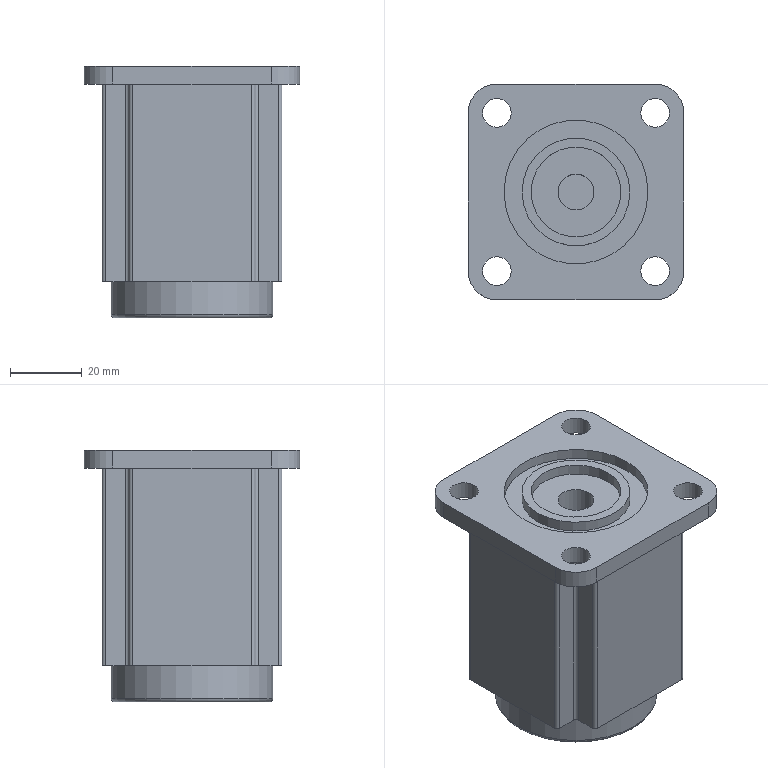Part | NX | features DATUM_CSYS 8, EXTRUDE 8, SKETCH 7, BLEND 2 | 1 solid | 58 faces | box 60 x 60 x 70 mm | volume 149838 mm3 | cylinder 29 | plane 28 | torus 1 | commonest cylinder face diameters 2 x12 5 x4 8 x4 16 x4 10 x1 25 x1
STEP:
#1=CARTESIAN_POINT('',(19.,-14.,-55.));
#2=VERTEX_POINT('',#1);
#3=CARTESIAN_POINT('',(21.5,-14.,-55.));
#4=DIRECTION('',(0.,0.,1.));
#5=DIRECTION('',(-1.,0.,0.));
#6=AXIS2_PLACEMENT_3D('',#3,#4,#5);
#7=CIRCLE('',#6,2.5);
#8=EDGE_CURVE('',#2,#2,#7,.T.);
#9=ORIENTED_EDGE('',*,*,#8,.T.);
#10=EDGE_LOOP('',(#9));
#11=FACE_BOUND('',#10,.T.);
#12=CARTESIAN_POINT('',(19.,14.,-55.));
#13=VERTEX_POINT('',#12);
#14=CARTESIAN_POINT('',(21.5,14.,-55.));
#15=DIRECTION('',(0.,0.,-1.));
#16=DIRECTION('',(-1.,0.,0.));
#17=AXIS2_PLACEMENT_3D('',#14,#15,#16);
#18=CIRCLE('',#17,2.5);
#19=EDGE_CURVE('',#13,#13,#18,.T.);
#20=ORIENTED_EDGE('',*,*,#19,.F.);
#21=EDGE_LOOP('',(#20));
#22=FACE_BOUND('',#21,.T.);
#23=CARTESIAN_POINT('',(-19.,-14.,-55.));
#24=VERTEX_POINT('',#23);
#25=CARTESIAN_POINT('',(-21.5,-14.,-55.));
#26=DIRECTION('',(0.,0.,-1.));
#27=DIRECTION('',(1.,0.,0.));
#28=AXIS2_PLACEMENT_3D('',#25,#26,#27);
#29=CIRCLE('',#28,2.5);
#30=EDGE_CURVE('',#24,#24,#29,.T.);
#31=ORIENTED_EDGE('',*,*,#30,.F.);
#32=EDGE_LOOP('',(#31));
#33=FACE_BOUND('',#32,.T.);
#34=CARTESIAN_POINT('',(22.5,0.,-55.));
#35=VERTEX_POINT('',#34);
#36=CARTESIAN_POINT('',(0.,0.,-55.));
#37=DIRECTION('',(0.,0.,-1.));
#38=DIRECTION('',(1.,0.,0.));
#39=AXIS2_PLACEMENT_3D('',#36,#37,#38);
#40=CIRCLE('',#39,22.5);
#41=EDGE_CURVE('',#35,#35,#40,.T.);
#42=ORIENTED_EDGE('',*,*,#41,.F.);
#43=EDGE_LOOP('',(#42));
#44=FACE_BOUND('',#43,.T.);
#45=CARTESIAN_POINT('',(25.,16.5,-55.));
#46=VERTEX_POINT('',#45);
#47=CARTESIAN_POINT('',(25.,-16.5,-55.));
#48=VERTEX_POINT('',#47);
#49=CARTESIAN_POINT('',(25.,25.,-55.));
#50=DIRECTION('',(0.,-1.,0.));
#51=VECTOR('',#50,1000.);
#52=LINE('',#49,#51);
#53=EDGE_CURVE('',#46,#48,#52,.T.);
#54=ORIENTED_EDGE('',*,*,#53,.T.);
#55=CARTESIAN_POINT('',(24.,-17.5,-55.));
#56=VERTEX_POINT('',#55);
#57=CARTESIAN_POINT('',(24.,-16.5,-55.));
#58=DIRECTION('',(0.,0.,-1.));
#59=DIRECTION('',(-1.,0.,0.));
#60=AXIS2_PLACEMENT_3D('',#57,#58,#59);
#61=CIRCLE('',#60,1.);
#62=EDGE_CURVE('',#48,#56,#61,.T.);
#63=ORIENTED_EDGE('',*,*,#62,.T.);
#64=CARTESIAN_POINT('',(18.5,-17.5,-55.));
#65=VERTEX_POINT('',#64);
#66=CARTESIAN_POINT('',(17.5,-17.5,-55.));
#67=DIRECTION('',(1.,0.,0.));
#68=VECTOR('',#67,1000.);
#69=LINE('',#66,#68);
#70=EDGE_CURVE('',#65,#56,#69,.T.);
#71=ORIENTED_EDGE('',*,*,#70,.F.);
#72=CARTESIAN_POINT('',(17.5,-18.5,-55.));
#73=VERTEX_POINT('',#72);
#74=CARTESIAN_POINT('',(18.5,-18.5,-55.));
#75=DIRECTION('',(0.,0.,-1.));
#76=DIRECTION('',(-1.,0.,0.));
#77=AXIS2_PLACEMENT_3D('',#74,#75,#76);
#78=CIRCLE('',#77,1.);
#79=EDGE_CURVE('',#65,#73,#78,.F.);
#80=ORIENTED_EDGE('',*,*,#79,.T.);
#81=CARTESIAN_POINT('',(17.5,-24.,-55.));
#82=VERTEX_POINT('',#81);
#83=CARTESIAN_POINT('',(17.5,-25.,-55.));
#84=DIRECTION('',(0.,1.,0.));
#85=VECTOR('',#84,1000.);
#86=LINE('',#83,#85);
#87=EDGE_CURVE('',#82,#73,#86,.T.);
#88=ORIENTED_EDGE('',*,*,#87,.F.);
#89=CARTESIAN_POINT('',(16.5,-25.,-55.));
#90=VERTEX_POINT('',#89);
#91=CARTESIAN_POINT('',(16.5,-24.,-55.));
#92=DIRECTION('',(0.,0.,-1.));
#93=DIRECTION('',(-1.,0.,0.));
#94=AXIS2_PLACEMENT_3D('',#91,#92,#93);
#95=CIRCLE('',#94,1.);
#96=EDGE_CURVE('',#82,#90,#95,.T.);
#97=ORIENTED_EDGE('',*,*,#96,.T.);
#98=CARTESIAN_POINT('',(-16.5,-25.,-55.));
#99=VERTEX_POINT('',#98);
#100=CARTESIAN_POINT('',(25.,-25.,-55.));
#101=DIRECTION('',(-1.,0.,0.));
#102=VECTOR('',#101,1000.);
#103=LINE('',#100,#102);
#104=EDGE_CURVE('',#90,#99,#103,.T.);
#105=ORIENTED_EDGE('',*,*,#104,.T.);
#106=CARTESIAN_POINT('',(-17.5,-24.,-55.));
#107=VERTEX_POINT('',#106);
#108=CARTESIAN_POINT('',(-16.5,-24.,-55.));
#109=DIRECTION('',(0.,0.,-1.));
#110=DIRECTION('',(-1.,0.,0.));
#111=AXIS2_PLACEMENT_3D('',#108,#109,#110);
#112=CIRCLE('',#111,1.);
#113=EDGE_CURVE('',#99,#107,#112,.T.);
#114=ORIENTED_EDGE('',*,*,#113,.T.);
#115=CARTESIAN_POINT('',(-17.5,-18.5,-55.));
#116=VERTEX_POINT('',#115);
#117=CARTESIAN_POINT('',(-17.5,-17.5,-55.));
#118=DIRECTION('',(0.,-1.,0.));
#119=VECTOR('',#118,1000.);
#120=LINE('',#117,#119);
#121=EDGE_CURVE('',#116,#107,#120,.T.);
#122=ORIENTED_EDGE('',*,*,#121,.F.);
#123=CARTESIAN_POINT('',(-18.5,-17.5,-55.));
#124=VERTEX_POINT('',#123);
#125=CARTESIAN_POINT('',(-18.5,-18.5,-55.));
#126=DIRECTION('',(0.,0.,-1.));
#127=DIRECTION('',(-1.,0.,0.));
#128=AXIS2_PLACEMENT_3D('',#125,#126,#127);
#129=CIRCLE('',#128,1.);
#130=EDGE_CURVE('',#116,#124,#129,.F.);
#131=ORIENTED_EDGE('',*,*,#130,.T.);
#132=CARTESIAN_POINT('',(-24.,-17.5,-55.));
#133=VERTEX_POINT('',#132);
#134=CARTESIAN_POINT('',(-25.,-17.5,-55.));
#135=DIRECTION('',(1.,0.,0.));
#136=VECTOR('',#135,1000.);
#137=LINE('',#134,#136);
#138=EDGE_CURVE('',#133,#124,#137,.T.);
#139=ORIENTED_EDGE('',*,*,#138,.F.);
#140=CARTESIAN_POINT('',(-25.,-16.5,-55.));
#141=VERTEX_POINT('',#140);
#142=CARTESIAN_POINT('',(-24.,-16.5,-55.));
#143=DIRECTION('',(0.,0.,-1.));
#144=DIRECTION('',(-1.,0.,0.));
#145=AXIS2_PLACEMENT_3D('',#142,#143,#144);
#146=CIRCLE('',#145,1.);
#147=EDGE_CURVE('',#133,#141,#146,.T.);
#148=ORIENTED_EDGE('',*,*,#147,.T.);
#149=CARTESIAN_POINT('',(-25.,16.5,-55.));
#150=VERTEX_POINT('',#149);
#151=CARTESIAN_POINT('',(-25.,-25.,-55.));
#152=DIRECTION('',(0.,1.,0.));
#153=VECTOR('',#152,1000.);
#154=LINE('',#151,#153);
#155=EDGE_CURVE('',#141,#150,#154,.T.);
#156=ORIENTED_EDGE('',*,*,#155,.T.);
#157=CARTESIAN_POINT('',(-24.,17.5,-55.));
#158=VERTEX_POINT('',#157);
#159=CARTESIAN_POINT('',(-24.,16.5,-55.));
#160=DIRECTION('',(0.,0.,-1.));
#161=DIRECTION('',(-1.,0.,0.));
#162=AXIS2_PLACEMENT_3D('',#159,#160,#161);
#163=CIRCLE('',#162,1.);
#164=EDGE_CURVE('',#150,#158,#163,.T.);
#165=ORIENTED_EDGE('',*,*,#164,.T.);
#166=CARTESIAN_POINT('',(-18.5,17.5,-55.));
#167=VERTEX_POINT('',#166);
#168=CARTESIAN_POINT('',(-17.5,17.5,-55.));
#169=DIRECTION('',(-1.,0.,0.));
#170=VECTOR('',#169,1000.);
#171=LINE('',#168,#170);
#172=EDGE_CURVE('',#167,#158,#171,.T.);
#173=ORIENTED_EDGE('',*,*,#172,.F.);
#174=CARTESIAN_POINT('',(-17.5,18.5,-55.));
#175=VERTEX_POINT('',#174);
#176=CARTESIAN_POINT('',(-18.5,18.5,-55.));
#177=DIRECTION('',(0.,0.,-1.));
#178=DIRECTION('',(-1.,0.,0.));
#179=AXIS2_PLACEMENT_3D('',#176,#177,#178);
#180=CIRCLE('',#179,1.);
#181=EDGE_CURVE('',#167,#175,#180,.F.);
#182=ORIENTED_EDGE('',*,*,#181,.T.);
#183=CARTESIAN_POINT('',(-17.5,24.,-55.));
#184=VERTEX_POINT('',#183);
#185=CARTESIAN_POINT('',(-17.5,25.,-55.));
#186=DIRECTION('',(0.,-1.,0.));
#187=VECTOR('',#186,1000.);
#188=LINE('',#185,#187);
#189=EDGE_CURVE('',#184,#175,#188,.T.);
#190=ORIENTED_EDGE('',*,*,#189,.F.);
#191=CARTESIAN_POINT('',(-16.5,25.,-55.));
#192=VERTEX_POINT('',#191);
#193=CARTESIAN_POINT('',(-16.5,24.,-55.));
#194=DIRECTION('',(0.,0.,-1.));
#195=DIRECTION('',(-1.,0.,0.));
#196=AXIS2_PLACEMENT_3D('',#193,#194,#195);
#197=CIRCLE('',#196,1.);
#198=EDGE_CURVE('',#184,#192,#197,.T.);
#199=ORIENTED_EDGE('',*,*,#198,.T.);
#200=CARTESIAN_POINT('',(16.5,25.,-55.));
#201=VERTEX_POINT('',#200);
#202=CARTESIAN_POINT('',(-25.,25.,-55.));
#203=DIRECTION('',(1.,0.,0.));
#204=VECTOR('',#203,1000.);
#205=LINE('',#202,#204);
#206=EDGE_CURVE('',#192,#201,#205,.T.);
#207=ORIENTED_EDGE('',*,*,#206,.T.);
#208=CARTESIAN_POINT('',(17.5,24.,-55.));
#209=VERTEX_POINT('',#208);
#210=CARTESIAN_POINT('',(16.5,24.,-55.));
#211=DIRECTION('',(0.,0.,-1.));
#212=DIRECTION('',(-1.,0.,0.));
#213=AXIS2_PLACEMENT_3D('',#210,#211,#212);
#214=CIRCLE('',#213,1.);
#215=EDGE_CURVE('',#201,#209,#214,.T.);
#216=ORIENTED_EDGE('',*,*,#215,.T.);
#217=CARTESIAN_POINT('',(17.5,18.5,-55.));
#218=VERTEX_POINT('',#217);
#219=CARTESIAN_POINT('',(17.5,17.5,-55.));
#220=DIRECTION('',(0.,1.,0.));
#221=VECTOR('',#220,1000.);
#222=LINE('',#219,#221);
#223=EDGE_CURVE('',#218,#209,#222,.T.);
#224=ORIENTED_EDGE('',*,*,#223,.F.);
#225=CARTESIAN_POINT('',(18.5,17.5,-55.));
#226=VERTEX_POINT('',#225);
#227=CARTESIAN_POINT('',(18.5,18.5,-55.));
#228=DIRECTION('',(0.,0.,-1.));
#229=DIRECTION('',(-1.,0.,0.));
#230=AXIS2_PLACEMENT_3D('',#227,#228,#229);
#231=CIRCLE('',#230,1.);
#232=EDGE_CURVE('',#218,#226,#231,.F.);
#233=ORIENTED_EDGE('',*,*,#232,.T.);
#234=CARTESIAN_POINT('',(24.,17.5,-55.));
#235=VERTEX_POINT('',#234);
#236=CARTESIAN_POINT('',(25.,17.5,-55.));
#237=DIRECTION('',(-1.,0.,0.));
#238=VECTOR('',#237,1000.);
#239=LINE('',#236,#238);
#240=EDGE_CURVE('',#235,#226,#239,.T.);
#241=ORIENTED_EDGE('',*,*,#240,.F.);
#242=CARTESIAN_POINT('',(24.,16.5,-55.));
#243=DIRECTION('',(0.,0.,-1.));
#244=DIRECTION('',(-1.,0.,0.));
#245=AXIS2_PLACEMENT_3D('',#242,#243,#244);
#246=CIRCLE('',#245,1.);
#247=EDGE_CURVE('',#235,#46,#246,.T.);
#248=ORIENTED_EDGE('',*,*,#247,.T.);
#249=EDGE_LOOP('',(#54,#63,#71,#80,#88,#97,#105,#114,#122,#131,#139,#148,#156,#165,#173,#182,#190,#199,#207,#216,#224,#233,#241,#248));
#250=FACE_BOUND('',#249,.T.);
#251=CARTESIAN_POINT('',(-19.,14.,-55.));
#252=VERTEX_POINT('',#251);
#253=CARTESIAN_POINT('',(-21.5,14.,-55.));
#254=DIRECTION('',(0.,0.,1.));
#255=DIRECTION('',(1.,0.,0.));
#256=AXIS2_PLACEMENT_3D('',#253,#254,#255);
#257=CIRCLE('',#256,2.5);
#258=EDGE_CURVE('',#252,#252,#257,.T.);
#259=ORIENTED_EDGE('',*,*,#258,.T.);
#260=EDGE_LOOP('',(#259));
#261=FACE_BOUND('',#260,.T.);
#262=CARTESIAN_POINT('',(0.,0.,-55.));
#263=DIRECTION('',(0.,0.,-1.));
#264=DIRECTION('',(-1.,0.,0.));
#265=AXIS2_PLACEMENT_3D('',#262,#263,#264);
#266=PLANE('',#265);
#267=ADVANCED_FACE('',(#11,#22,#33,#44,#250,#261),#266,.T.);
#268=ORIENTED_EDGE('',*,*,#155,.F.);
#269=CARTESIAN_POINT('',(-25.,-16.5,0.));
#270=VERTEX_POINT('',#269);
#271=CARTESIAN_POINT('',(-25.,-16.5,-55.));
#272=DIRECTION('',(0.,0.,-1.));
#273=VECTOR('',#272,1000.);
#274=LINE('',#271,#273);
#275=EDGE_CURVE('',#141,#270,#274,.F.);
#276=ORIENTED_EDGE('',*,*,#275,.T.);
#277=CARTESIAN_POINT('',(-25.,16.5,0.));
#278=VERTEX_POINT('',#277);
#279=CARTESIAN_POINT('',(-25.,-25.,0.));
#280=DIRECTION('',(0.,1.,0.));
#281=VECTOR('',#280,1000.);
#282=LINE('',#279,#281);
#283=EDGE_CURVE('',#270,#278,#282,.T.);
#284=ORIENTED_EDGE('',*,*,#283,.T.);
#285=CARTESIAN_POINT('',(-25.,16.5,-55.));
#286=DIRECTION('',(0.,0.,-1.));
#287=VECTOR('',#286,1000.);
#288=LINE('',#285,#287);
#289=EDGE_CURVE('',#278,#150,#288,.T.);
#290=ORIENTED_EDGE('',*,*,#289,.T.);
#291=EDGE_LOOP('',(#268,#276,#284,#290));
#292=FACE_BOUND('',#291,.T.);
#293=CARTESIAN_POINT('',(-25.,-25.,-55.));
#294=DIRECTION('',(1.,0.,0.));
#295=DIRECTION('',(0.,1.,0.));
#296=AXIS2_PLACEMENT_3D('',#293,#294,#295);
#297=PLANE('',#296);
#298=ADVANCED_FACE('',(#292),#297,.F.);
#299=ORIENTED_EDGE('',*,*,#206,.F.);
#300=CARTESIAN_POINT('',(-16.5,25.,0.));
#301=VERTEX_POINT('',#300);
#302=CARTESIAN_POINT('',(-16.5,25.,-55.));
#303=DIRECTION('',(0.,0.,-1.));
#304=VECTOR('',#303,1000.);
#305=LINE('',#302,#304);
#306=EDGE_CURVE('',#192,#301,#305,.F.);
#307=ORIENTED_EDGE('',*,*,#306,.T.);
#308=CARTESIAN_POINT('',(16.5,25.,0.));
#309=VERTEX_POINT('',#308);
#310=CARTESIAN_POINT('',(-25.,25.,0.));
#311=DIRECTION('',(1.,0.,0.));
#312=VECTOR('',#311,1000.);
#313=LINE('',#310,#312);
#314=EDGE_CURVE('',#301,#309,#313,.T.);
#315=ORIENTED_EDGE('',*,*,#314,.T.);
#316=CARTESIAN_POINT('',(16.5,25.,-55.));
#317=DIRECTION('',(0.,0.,-1.));
#318=VECTOR('',#317,1000.);
#319=LINE('',#316,#318);
#320=EDGE_CURVE('',#309,#201,#319,.T.);
#321=ORIENTED_EDGE('',*,*,#320,.T.);
#322=EDGE_LOOP('',(#299,#307,#315,#321));
#323=FACE_BOUND('',#322,.T.);
#324=CARTESIAN_POINT('',(-25.,25.,-55.));
#325=DIRECTION('',(0.,-1.,0.));
#326=DIRECTION('',(1.,0.,0.));
#327=AXIS2_PLACEMENT_3D('',#324,#325,#326);
#328=PLANE('',#327);
#329=ADVANCED_FACE('',(#323),#328,.F.);
#330=CARTESIAN_POINT('',(25.,16.5,0.));
#331=VERTEX_POINT('',#330);
#332=CARTESIAN_POINT('',(25.,-16.5,0.));
#333=VERTEX_POINT('',#332);
#334=CARTESIAN_POINT('',(25.,25.,0.));
#335=DIRECTION('',(0.,-1.,0.));
#336=VECTOR('',#335,1000.);
#337=LINE('',#334,#336);
#338=EDGE_CURVE('',#331,#333,#337,.T.);
#339=ORIENTED_EDGE('',*,*,#338,.T.);
#340=CARTESIAN_POINT('',(25.,-16.5,-55.));
#341=DIRECTION('',(0.,0.,-1.));
#342=VECTOR('',#341,1000.);
#343=LINE('',#340,#342);
#344=EDGE_CURVE('',#333,#48,#343,.T.);
#345=ORIENTED_EDGE('',*,*,#344,.T.);
#346=ORIENTED_EDGE('',*,*,#53,.F.);
#347=CARTESIAN_POINT('',(25.,16.5,-55.));
#348=DIRECTION('',(0.,0.,-1.));
#349=VECTOR('',#348,1000.);
#350=LINE('',#347,#349);
#351=EDGE_CURVE('',#46,#331,#350,.F.);
#352=ORIENTED_EDGE('',*,*,#351,.T.);
#353=EDGE_LOOP('',(#339,#345,#346,#352));
#354=FACE_BOUND('',#353,.T.);
#355=CARTESIAN_POINT('',(25.,25.,-55.));
#356=DIRECTION('',(-1.,0.,0.));
#357=DIRECTION('',(0.,-1.,0.));
#358=AXIS2_PLACEMENT_3D('',#355,#356,#357);
#359=PLANE('',#358);
#360=ADVANCED_FACE('',(#354),#359,.F.);
#361=ORIENTED_EDGE('',*,*,#104,.F.);
#362=CARTESIAN_POINT('',(16.5,-25.,0.));
#363=VERTEX_POINT('',#362);
#364=CARTESIAN_POINT('',(16.5,-25.,-55.));
#365=DIRECTION('',(0.,0.,-1.));
#366=VECTOR('',#365,1000.);
#367=LINE('',#364,#366);
#368=EDGE_CURVE('',#90,#363,#367,.F.);
#369=ORIENTED_EDGE('',*,*,#368,.T.);
#370=CARTESIAN_POINT('',(-16.5,-25.,0.));
#371=VERTEX_POINT('',#370);
#372=CARTESIAN_POINT('',(25.,-25.,0.));
#373=DIRECTION('',(-1.,0.,0.));
#374=VECTOR('',#373,1000.);
#375=LINE('',#372,#374);
#376=EDGE_CURVE('',#363,#371,#375,.T.);
#377=ORIENTED_EDGE('',*,*,#376,.T.);
#378=CARTESIAN_POINT('',(-16.5,-25.,-55.));
#379=DIRECTION('',(0.,0.,-1.));
#380=VECTOR('',#379,1000.);
#381=LINE('',#378,#380);
#382=EDGE_CURVE('',#371,#99,#381,.T.);
#383=ORIENTED_EDGE('',*,*,#382,.T.);
#384=EDGE_LOOP('',(#361,#369,#377,#383));
#385=FACE_BOUND('',#384,.T.);
#386=CARTESIAN_POINT('',(25.,-25.,-55.));
#387=DIRECTION('',(0.,1.,0.));
#388=DIRECTION('',(-1.,0.,0.));
#389=AXIS2_PLACEMENT_3D('',#386,#387,#388);
#390=PLANE('',#389);
#391=ADVANCED_FACE('',(#385),#390,.F.);
#392=CARTESIAN_POINT('',(-26.,22.,0.));
#393=VERTEX_POINT('',#392);
#394=CARTESIAN_POINT('',(-22.,22.,0.));
#395=DIRECTION('',(0.,0.,-1.));
#396=DIRECTION('',(-1.,0.,0.));
#397=AXIS2_PLACEMENT_3D('',#394,#395,#396);
#398=CIRCLE('',#397,4.);
#399=EDGE_CURVE('',#393,#393,#398,.T.);
#400=ORIENTED_EDGE('',*,*,#399,.F.);
#401=EDGE_LOOP('',(#400));
#402=FACE_BOUND('',#401,.T.);
#403=CARTESIAN_POINT('',(17.5,-24.,0.));
#404=VERTEX_POINT('',#403);
#405=CARTESIAN_POINT('',(17.5,-18.5,0.));
#406=VERTEX_POINT('',#405);
#407=CARTESIAN_POINT('',(17.5,-25.,0.));
#408=DIRECTION('',(0.,1.,0.));
#409=VECTOR('',#408,1000.);
#410=LINE('',#407,#409);
#411=EDGE_CURVE('',#404,#406,#410,.T.);
#412=ORIENTED_EDGE('',*,*,#411,.T.);
#413=CARTESIAN_POINT('',(18.5,-17.5,0.));
#414=VERTEX_POINT('',#413);
#415=CARTESIAN_POINT('',(18.5,-18.5,0.));
#416=DIRECTION('',(0.,0.,1.));
#417=DIRECTION('',(1.,0.,0.));
#418=AXIS2_PLACEMENT_3D('',#415,#416,#417);
#419=CIRCLE('',#418,1.);
#420=EDGE_CURVE('',#406,#414,#419,.F.);
#421=ORIENTED_EDGE('',*,*,#420,.T.);
#422=CARTESIAN_POINT('',(24.,-17.5,0.));
#423=VERTEX_POINT('',#422);
#424=CARTESIAN_POINT('',(17.5,-17.5,0.));
#425=DIRECTION('',(1.,0.,0.));
#426=VECTOR('',#425,1000.);
#427=LINE('',#424,#426);
#428=EDGE_CURVE('',#414,#423,#427,.T.);
#429=ORIENTED_EDGE('',*,*,#428,.T.);
#430=CARTESIAN_POINT('',(24.,-16.5,0.));
#431=DIRECTION('',(0.,0.,1.));
#432=DIRECTION('',(1.,0.,0.));
#433=AXIS2_PLACEMENT_3D('',#430,#431,#432);
#434=CIRCLE('',#433,1.);
#435=EDGE_CURVE('',#423,#333,#434,.T.);
#436=ORIENTED_EDGE('',*,*,#435,.T.);
#437=ORIENTED_EDGE('',*,*,#338,.F.);
#438=CARTESIAN_POINT('',(24.,17.5,0.));
#439=VERTEX_POINT('',#438);
#440=CARTESIAN_POINT('',(24.,16.5,0.));
#441=DIRECTION('',(0.,0.,1.));
#442=DIRECTION('',(1.,0.,0.));
#443=AXIS2_PLACEMENT_3D('',#440,#441,#442);
#444=CIRCLE('',#443,1.);
#445=EDGE_CURVE('',#331,#439,#444,.T.);
#446=ORIENTED_EDGE('',*,*,#445,.T.);
#447=CARTESIAN_POINT('',(18.5,17.5,0.));
#448=VERTEX_POINT('',#447);
#449=CARTESIAN_POINT('',(25.,17.5,0.));
#450=DIRECTION('',(-1.,0.,0.));
#451=VECTOR('',#450,1000.);
#452=LINE('',#449,#451);
#453=EDGE_CURVE('',#439,#448,#452,.T.);
#454=ORIENTED_EDGE('',*,*,#453,.T.);
#455=CARTESIAN_POINT('',(17.5,18.5,0.));
#456=VERTEX_POINT('',#455);
#457=CARTESIAN_POINT('',(18.5,18.5,0.));
#458=DIRECTION('',(0.,0.,1.));
#459=DIRECTION('',(1.,0.,0.));
#460=AXIS2_PLACEMENT_3D('',#457,#458,#459);
#461=CIRCLE('',#460,1.);
#462=EDGE_CURVE('',#448,#456,#461,.F.);
#463=ORIENTED_EDGE('',*,*,#462,.T.);
#464=CARTESIAN_POINT('',(17.5,24.,0.));
#465=VERTEX_POINT('',#464);
#466=CARTESIAN_POINT('',(17.5,17.5,0.));
#467=DIRECTION('',(0.,1.,0.));
#468=VECTOR('',#467,1000.);
#469=LINE('',#466,#468);
#470=EDGE_CURVE('',#456,#465,#469,.T.);
#471=ORIENTED_EDGE('',*,*,#470,.T.);
#472=CARTESIAN_POINT('',(16.5,24.,0.));
#473=DIRECTION('',(0.,0.,1.));
#474=DIRECTION('',(1.,0.,0.));
#475=AXIS2_PLACEMENT_3D('',#472,#473,#474);
#476=CIRCLE('',#475,1.);
#477=EDGE_CURVE('',#465,#309,#476,.T.);
#478=ORIENTED_EDGE('',*,*,#477,.T.);
#479=ORIENTED_EDGE('',*,*,#314,.F.);
#480=CARTESIAN_POINT('',(-17.5,24.,0.));
#481=VERTEX_POINT('',#480);
#482=CARTESIAN_POINT('',(-16.5,24.,0.));
#483=DIRECTION('',(0.,0.,1.));
#484=DIRECTION('',(1.,0.,0.));
#485=AXIS2_PLACEMENT_3D('',#482,#483,#484);
#486=CIRCLE('',#485,1.);
#487=EDGE_CURVE('',#301,#481,#486,.T.);
#488=ORIENTED_EDGE('',*,*,#487,.T.);
#489=CARTESIAN_POINT('',(-17.5,18.5,0.));
#490=VERTEX_POINT('',#489);
#491=CARTESIAN_POINT('',(-17.5,25.,0.));
#492=DIRECTION('',(0.,-1.,0.));
#493=VECTOR('',#492,1000.);
#494=LINE('',#491,#493);
#495=EDGE_CURVE('',#481,#490,#494,.T.);
#496=ORIENTED_EDGE('',*,*,#495,.T.);
#497=CARTESIAN_POINT('',(-18.5,17.5,0.));
#498=VERTEX_POINT('',#497);
#499=CARTESIAN_POINT('',(-18.5,18.5,0.));
#500=DIRECTION('',(0.,0.,1.));
#501=DIRECTION('',(1.,0.,0.));
#502=AXIS2_PLACEMENT_3D('',#499,#500,#501);
#503=CIRCLE('',#502,1.);
#504=EDGE_CURVE('',#490,#498,#503,.F.);
#505=ORIENTED_EDGE('',*,*,#504,.T.);
#506=CARTESIAN_POINT('',(-24.,17.5,0.));
#507=VERTEX_POINT('',#506);
#508=CARTESIAN_POINT('',(-17.5,17.5,0.));
#509=DIRECTION('',(-1.,0.,0.));
#510=VECTOR('',#509,1000.);
#511=LINE('',#508,#510);
#512=EDGE_CURVE('',#498,#507,#511,.T.);
#513=ORIENTED_EDGE('',*,*,#512,.T.);
#514=CARTESIAN_POINT('',(-24.,16.5,0.));
#515=DIRECTION('',(0.,0.,1.));
#516=DIRECTION('',(1.,0.,0.));
#517=AXIS2_PLACEMENT_3D('',#514,#515,#516);
#518=CIRCLE('',#517,1.);
#519=EDGE_CURVE('',#507,#278,#518,.T.);
#520=ORIENTED_EDGE('',*,*,#519,.T.);
#521=ORIENTED_EDGE('',*,*,#283,.F.);
#522=CARTESIAN_POINT('',(-24.,-17.5,0.));
#523=VERTEX_POINT('',#522);
#524=CARTESIAN_POINT('',(-24.,-16.5,0.));
#525=DIRECTION('',(0.,0.,1.));
#526=DIRECTION('',(1.,0.,0.));
#527=AXIS2_PLACEMENT_3D('',#524,#525,#526);
#528=CIRCLE('',#527,1.);
#529=EDGE_CURVE('',#270,#523,#528,.T.);
#530=ORIENTED_EDGE('',*,*,#529,.T.);
#531=CARTESIAN_POINT('',(-18.5,-17.5,0.));
#532=VERTEX_POINT('',#531);
#533=CARTESIAN_POINT('',(-25.,-17.5,0.));
#534=DIRECTION('',(1.,0.,0.));
#535=VECTOR('',#534,1000.);
#536=LINE('',#533,#535);
#537=EDGE_CURVE('',#523,#532,#536,.T.);
#538=ORIENTED_EDGE('',*,*,#537,.T.);
#539=CARTESIAN_POINT('',(-17.5,-18.5,0.));
#540=VERTEX_POINT('',#539);
#541=CARTESIAN_POINT('',(-18.5,-18.5,0.));
#542=DIRECTION('',(0.,0.,1.));
#543=DIRECTION('',(1.,0.,0.));
#544=AXIS2_PLACEMENT_3D('',#541,#542,#543);
#545=CIRCLE('',#544,1.);
#546=EDGE_CURVE('',#532,#540,#545,.F.);
#547=ORIENTED_EDGE('',*,*,#546,.T.);
#548=CARTESIAN_POINT('',(-17.5,-24.,0.));
#549=VERTEX_POINT('',#548);
#550=CARTESIAN_POINT('',(-17.5,-17.5,0.));
#551=DIRECTION('',(0.,-1.,0.));
#552=VECTOR('',#551,1000.);
#553=LINE('',#550,#552);
#554=EDGE_CURVE('',#540,#549,#553,.T.);
#555=ORIENTED_EDGE('',*,*,#554,.T.);
#556=CARTESIAN_POINT('',(-16.5,-24.,0.));
#557=DIRECTION('',(0.,0.,1.));
#558=DIRECTION('',(1.,0.,0.));
#559=AXIS2_PLACEMENT_3D('',#556,#557,#558);
#560=CIRCLE('',#559,1.);
#561=EDGE_CURVE('',#549,#371,#560,.T.);
#562=ORIENTED_EDGE('',*,*,#561,.T.);
#563=ORIENTED_EDGE('',*,*,#376,.F.);
#564=CARTESIAN_POINT('',(16.5,-24.,0.));
#565=DIRECTION('',(0.,0.,1.));
#566=DIRECTION('',(1.,0.,0.));
#567=AXIS2_PLACEMENT_3D('',#564,#565,#566);
#568=CIRCLE('',#567,1.);
#569=EDGE_CURVE('',#363,#404,#568,.T.);
#570=ORIENTED_EDGE('',*,*,#569,.T.);
#571=EDGE_LOOP('',(#412,#421,#429,#436,#437,#446,#454,#463,#471,#478,#479,#488,#496,#505,#513,#520,#521,#530,#538,#547,#555,#562,#563,#570));
#572=FACE_BOUND('',#571,.T.);
#573=CARTESIAN_POINT('',(26.,-22.,0.));
#574=VERTEX_POINT('',#573);
#575=CARTESIAN_POINT('',(22.,-22.,0.));
#576=DIRECTION('',(0.,0.,-1.));
#577=DIRECTION('',(1.,0.,0.));
#578=AXIS2_PLACEMENT_3D('',#575,#576,#577);
#579=CIRCLE('',#578,4.);
#580=EDGE_CURVE('',#574,#574,#579,.T.);
#581=ORIENTED_EDGE('',*,*,#580,.F.);
#582=EDGE_LOOP('',(#581));
#583=FACE_BOUND('',#582,.T.);
#584=CARTESIAN_POINT('',(26.,22.,0.));
#585=VERTEX_POINT('',#584);
#586=CARTESIAN_POINT('',(22.,22.,0.));
#587=DIRECTION('',(0.,0.,1.));
#588=DIRECTION('',(1.,0.,0.));
#589=AXIS2_PLACEMENT_3D('',#586,#587,#588);
#590=CIRCLE('',#589,4.);
#591=EDGE_CURVE('',#585,#585,#590,.T.);
#592=ORIENTED_EDGE('',*,*,#591,.T.);
#593=EDGE_LOOP('',(#592));
#594=FACE_BOUND('',#593,.T.);
#595=CARTESIAN_POINT('',(-26.,-22.,0.));
#596=VERTEX_POINT('',#595);
#597=CARTESIAN_POINT('',(-22.,-22.,0.));
#598=DIRECTION('',(0.,0.,1.));
#599=DIRECTION('',(-1.,0.,0.));
#600=AXIS2_PLACEMENT_3D('',#597,#598,#599);
#601=CIRCLE('',#600,4.);
#602=EDGE_CURVE('',#596,#596,#601,.T.);
#603=ORIENTED_EDGE('',*,*,#602,.T.);
#604=EDGE_LOOP('',(#603));
#605=FACE_BOUND('',#604,.T.);
#606=CARTESIAN_POINT('',(-30.,22.,0.));
#607=VERTEX_POINT('',#606);
#608=CARTESIAN_POINT('',(-30.,-22.,0.));
#609=VERTEX_POINT('',#608);
#610=CARTESIAN_POINT('',(-30.,22.,0.));
#611=DIRECTION('',(0.,-1.,0.));
#612=VECTOR('',#611,1000.);
#613=LINE('',#610,#612);
#614=EDGE_CURVE('',#607,#609,#613,.T.);
#615=ORIENTED_EDGE('',*,*,#614,.F.);
#616=CARTESIAN_POINT('',(-22.,30.,0.));
#617=VERTEX_POINT('',#616);
#618=CARTESIAN_POINT('',(-22.,22.,0.));
#619=DIRECTION('',(0.,0.,1.));
#620=DIRECTION('',(1.,0.,0.));
#621=AXIS2_PLACEMENT_3D('',#618,#619,#620);
#622=CIRCLE('',#621,8.);
#623=EDGE_CURVE('',#617,#607,#622,.T.);
#624=ORIENTED_EDGE('',*,*,#623,.F.);
#625=CARTESIAN_POINT('',(22.,30.,0.));
#626=VERTEX_POINT('',#625);
#627=CARTESIAN_POINT('',(22.,30.,0.));
#628=DIRECTION('',(-1.,0.,0.));
#629=VECTOR('',#628,1000.);
#630=LINE('',#627,#629);
#631=EDGE_CURVE('',#626,#617,#630,.T.);
#632=ORIENTED_EDGE('',*,*,#631,.F.);
#633=CARTESIAN_POINT('',(30.,22.,0.));
#634=VERTEX_POINT('',#633);
#635=CARTESIAN_POINT('',(22.,22.,0.));
#636=DIRECTION('',(0.,0.,1.));
#637=DIRECTION('',(1.,0.,0.));
#638=AXIS2_PLACEMENT_3D('',#635,#636,#637);
#639=CIRCLE('',#638,8.);
#640=EDGE_CURVE('',#634,#626,#639,.T.);
#641=ORIENTED_EDGE('',*,*,#640,.F.);
#642=CARTESIAN_POINT('',(30.,-22.,0.));
#643=VERTEX_POINT('',#642);
#644=CARTESIAN_POINT('',(30.,-22.,0.));
#645=DIRECTION('',(0.,1.,0.));
#646=VECTOR('',#645,1000.);
#647=LINE('',#644,#646);
#648=EDGE_CURVE('',#643,#634,#647,.T.);
#649=ORIENTED_EDGE('',*,*,#648,.F.);
#650=CARTESIAN_POINT('',(22.,-30.,0.));
#651=VERTEX_POINT('',#650);
#652=CARTESIAN_POINT('',(22.,-22.,0.));
#653=DIRECTION('',(0.,0.,1.));
#654=DIRECTION('',(1.,0.,0.));
#655=AXIS2_PLACEMENT_3D('',#652,#653,#654);
#656=CIRCLE('',#655,8.);
#657=EDGE_CURVE('',#651,#643,#656,.T.);
#658=ORIENTED_EDGE('',*,*,#657,.F.);
#659=CARTESIAN_POINT('',(-22.,-30.,0.));
#660=VERTEX_POINT('',#659);
#661=CARTESIAN_POINT('',(-22.,-30.,0.));
#662=DIRECTION('',(1.,0.,0.));
#663=VECTOR('',#662,1000.);
#664=LINE('',#661,#663);
#665=EDGE_CURVE('',#660,#651,#664,.T.);
#666=ORIENTED_EDGE('',*,*,#665,.F.);
#667=CARTESIAN_POINT('',(-22.,-22.,0.));
#668=DIRECTION('',(0.,0.,1.));
#669=DIRECTION('',(1.,0.,0.));
#670=AXIS2_PLACEMENT_3D('',#667,#668,#669);
#671=CIRCLE('',#670,8.);
#672=EDGE_CURVE('',#609,#660,#671,.T.);
#673=ORIENTED_EDGE('',*,*,#672,.F.);
#674=EDGE_LOOP('',(#615,#624,#632,#641,#649,#658,#666,#673));
#675=FACE_BOUND('',#674,.T.);
#676=CARTESIAN_POINT('',(-22.,-22.,0.));
#677=DIRECTION('',(0.,0.,1.));
#678=DIRECTION('',(1.,0.,0.));
#679=AXIS2_PLACEMENT_3D('',#676,#677,#678);
#680=PLANE('',#679);
#681=ADVANCED_FACE('',(#402,#572,#583,#594,#605,#675),#680,.F.);
#682=ORIENTED_EDGE('',*,*,#614,.T.);
#683=CARTESIAN_POINT('',(-30.,-22.,5.));
#684=VERTEX_POINT('',#683);
#685=CARTESIAN_POINT('',(-30.,-22.,5.));
#686=DIRECTION('',(0.,0.,-1.));
#687=VECTOR('',#686,1000.);
#688=LINE('',#685,#687);
#689=EDGE_CURVE('',#684,#609,#688,.T.);
#690=ORIENTED_EDGE('',*,*,#689,.F.);
#691=CARTESIAN_POINT('',(-30.,22.,5.));
#692=VERTEX_POINT('',#691);
#693=CARTESIAN_POINT('',(-30.,22.,5.));
#694=DIRECTION('',(0.,-1.,0.));
#695=VECTOR('',#694,1000.);
#696=LINE('',#693,#695);
#697=EDGE_CURVE('',#692,#684,#696,.T.);
#698=ORIENTED_EDGE('',*,*,#697,.F.);
#699=CARTESIAN_POINT('',(-30.,22.,5.));
#700=DIRECTION('',(0.,0.,-1.));
#701=VECTOR('',#700,1000.);
#702=LINE('',#699,#701);
#703=EDGE_CURVE('',#692,#607,#702,.T.);
#704=ORIENTED_EDGE('',*,*,#703,.T.);
#705=EDGE_LOOP('',(#682,#690,#698,#704));
#706=FACE_BOUND('',#705,.T.);
#707=CARTESIAN_POINT('',(-30.,22.,5.));
#708=DIRECTION('',(1.,0.,0.));
#709=DIRECTION('',(0.,1.,0.));
#710=AXIS2_PLACEMENT_3D('',#707,#708,#709);
#711=PLANE('',#710);
#712=ADVANCED_FACE('',(#706),#711,.F.);
#713=ORIENTED_EDGE('',*,*,#672,.T.);
#714=CARTESIAN_POINT('',(-22.,-30.,5.));
#715=VERTEX_POINT('',#714);
#716=CARTESIAN_POINT('',(-22.,-30.,5.));
#717=DIRECTION('',(0.,0.,-1.));
#718=VECTOR('',#717,1000.);
#719=LINE('',#716,#718);
#720=EDGE_CURVE('',#715,#660,#719,.T.);
#721=ORIENTED_EDGE('',*,*,#720,.F.);
#722=CARTESIAN_POINT('',(-22.,-22.,5.));
#723=DIRECTION('',(0.,0.,1.));
#724=DIRECTION('',(1.,0.,0.));
#725=AXIS2_PLACEMENT_3D('',#722,#723,#724);
#726=CIRCLE('',#725,8.);
#727=EDGE_CURVE('',#684,#715,#726,.T.);
#728=ORIENTED_EDGE('',*,*,#727,.F.);
#729=ORIENTED_EDGE('',*,*,#689,.T.);
#730=EDGE_LOOP('',(#713,#721,#728,#729));
#731=FACE_BOUND('',#730,.T.);
#732=CARTESIAN_POINT('',(-22.,-22.,5.));
#733=DIRECTION('',(0.,0.,-1.));
#734=DIRECTION('',(-1.,0.,0.));
#735=AXIS2_PLACEMENT_3D('',#732,#733,#734);
#736=CYLINDRICAL_SURFACE('',#735,8.);
#737=ADVANCED_FACE('',(#731),#736,.T.);
#738=ORIENTED_EDGE('',*,*,#665,.T.);
#739=CARTESIAN_POINT('',(22.,-30.,5.));
#740=VERTEX_POINT('',#739);
#741=CARTESIAN_POINT('',(22.,-30.,5.));
#742=DIRECTION('',(0.,0.,-1.));
#743=VECTOR('',#742,1000.);
#744=LINE('',#741,#743);
#745=EDGE_CURVE('',#740,#651,#744,.T.);
#746=ORIENTED_EDGE('',*,*,#745,.F.);
#747=CARTESIAN_POINT('',(-22.,-30.,5.));
#748=DIRECTION('',(1.,0.,0.));
#749=VECTOR('',#748,1000.);
#750=LINE('',#747,#749);
#751=EDGE_CURVE('',#715,#740,#750,.T.);
#752=ORIENTED_EDGE('',*,*,#751,.F.);
#753=ORIENTED_EDGE('',*,*,#720,.T.);
#754=EDGE_LOOP('',(#738,#746,#752,#753));
#755=FACE_BOUND('',#754,.T.);
#756=CARTESIAN_POINT('',(-22.,-30.,5.));
#757=DIRECTION('',(0.,1.,0.));
#758=DIRECTION('',(0.,0.,1.));
#759=AXIS2_PLACEMENT_3D('',#756,#757,#758);
#760=PLANE('',#759);
#761=ADVANCED_FACE('',(#755),#760,.F.);
#762=ORIENTED_EDGE('',*,*,#657,.T.);
#763=CARTESIAN_POINT('',(30.,-22.,5.));
#764=VERTEX_POINT('',#763);
#765=CARTESIAN_POINT('',(30.,-22.,5.));
#766=DIRECTION('',(0.,0.,-1.));
#767=VECTOR('',#766,1000.);
#768=LINE('',#765,#767);
#769=EDGE_CURVE('',#764,#643,#768,.T.);
#770=ORIENTED_EDGE('',*,*,#769,.F.);
#771=CARTESIAN_POINT('',(22.,-22.,5.));
#772=DIRECTION('',(0.,0.,1.));
#773=DIRECTION('',(1.,0.,0.));
#774=AXIS2_PLACEMENT_3D('',#771,#772,#773);
#775=CIRCLE('',#774,8.);
#776=EDGE_CURVE('',#740,#764,#775,.T.);
#777=ORIENTED_EDGE('',*,*,#776,.F.);
#778=ORIENTED_EDGE('',*,*,#745,.T.);
#779=EDGE_LOOP('',(#762,#770,#777,#778));
#780=FACE_BOUND('',#779,.T.);
#781=CARTESIAN_POINT('',(22.,-22.,5.));
#782=DIRECTION('',(0.,0.,-1.));
#783=DIRECTION('',(-1.,0.,0.));
#784=AXIS2_PLACEMENT_3D('',#781,#782,#783);
#785=CYLINDRICAL_SURFACE('',#784,8.);
#786=ADVANCED_FACE('',(#780),#785,.T.);
#787=ORIENTED_EDGE('',*,*,#648,.T.);
#788=CARTESIAN_POINT('',(30.,22.,5.));
#789=VERTEX_POINT('',#788);
#790=CARTESIAN_POINT('',(30.,22.,5.));
#791=DIRECTION('',(0.,0.,-1.));
#792=VECTOR('',#791,1000.);
#793=LINE('',#790,#792);
#794=EDGE_CURVE('',#789,#634,#793,.T.);
#795=ORIENTED_EDGE('',*,*,#794,.F.);
#796=CARTESIAN_POINT('',(30.,-22.,5.));
#797=DIRECTION('',(0.,1.,0.));
#798=VECTOR('',#797,1000.);
#799=LINE('',#796,#798);
#800=EDGE_CURVE('',#764,#789,#799,.T.);
#801=ORIENTED_EDGE('',*,*,#800,.F.);
#802=ORIENTED_EDGE('',*,*,#769,.T.);
#803=EDGE_LOOP('',(#787,#795,#801,#802));
#804=FACE_BOUND('',#803,.T.);
#805=CARTESIAN_POINT('',(30.,-22.,5.));
#806=DIRECTION('',(-1.,0.,0.));
#807=DIRECTION('',(0.,-1.,0.));
#808=AXIS2_PLACEMENT_3D('',#805,#806,#807);
#809=PLANE('',#808);
#810=ADVANCED_FACE('',(#804),#809,.F.);
#811=ORIENTED_EDGE('',*,*,#640,.T.);
#812=CARTESIAN_POINT('',(22.,30.,5.));
#813=VERTEX_POINT('',#812);
#814=CARTESIAN_POINT('',(22.,30.,5.));
#815=DIRECTION('',(0.,0.,-1.));
#816=VECTOR('',#815,1000.);
#817=LINE('',#814,#816);
#818=EDGE_CURVE('',#813,#626,#817,.T.);
#819=ORIENTED_EDGE('',*,*,#818,.F.);
#820=CARTESIAN_POINT('',(22.,22.,5.));
#821=DIRECTION('',(0.,0.,1.));
#822=DIRECTION('',(1.,0.,0.));
#823=AXIS2_PLACEMENT_3D('',#820,#821,#822);
#824=CIRCLE('',#823,8.);
#825=EDGE_CURVE('',#789,#813,#824,.T.);
#826=ORIENTED_EDGE('',*,*,#825,.F.);
#827=ORIENTED_EDGE('',*,*,#794,.T.);
#828=EDGE_LOOP('',(#811,#819,#826,#827));
#829=FACE_BOUND('',#828,.T.);
#830=CARTESIAN_POINT('',(22.,22.,5.));
#831=DIRECTION('',(0.,0.,-1.));
#832=DIRECTION('',(-1.,0.,0.));
#833=AXIS2_PLACEMENT_3D('',#830,#831,#832);
#834=CYLINDRICAL_SURFACE('',#833,8.);
#835=ADVANCED_FACE('',(#829),#834,.T.);
#836=ORIENTED_EDGE('',*,*,#631,.T.);
#837=CARTESIAN_POINT('',(-22.,30.,5.));
#838=VERTEX_POINT('',#837);
#839=CARTESIAN_POINT('',(-22.,30.,5.));
#840=DIRECTION('',(0.,0.,-1.));
#841=VECTOR('',#840,1000.);
#842=LINE('',#839,#841);
#843=EDGE_CURVE('',#838,#617,#842,.T.);
#844=ORIENTED_EDGE('',*,*,#843,.F.);
#845=CARTESIAN_POINT('',(22.,30.,5.));
#846=DIRECTION('',(-1.,0.,0.));
#847=VECTOR('',#846,1000.);
#848=LINE('',#845,#847);
#849=EDGE_CURVE('',#813,#838,#848,.T.);
#850=ORIENTED_EDGE('',*,*,#849,.F.);
#851=ORIENTED_EDGE('',*,*,#818,.T.);
#852=EDGE_LOOP('',(#836,#844,#850,#851));
#853=FACE_BOUND('',#852,.T.);
#854=CARTESIAN_POINT('',(22.,30.,5.));
#855=DIRECTION('',(0.,-1.,0.));
#856=DIRECTION('',(0.,0.,-1.));
#857=AXIS2_PLACEMENT_3D('',#854,#855,#856);
#858=PLANE('',#857);
#859=ADVANCED_FACE('',(#853),#858,.F.);
#860=CARTESIAN_POINT('',(-26.,22.,5.));
#861=VERTEX_POINT('',#860);
#862=CARTESIAN_POINT('',(-22.,22.,5.));
#863=DIRECTION('',(0.,0.,-1.));
#864=DIRECTION('',(-1.,0.,0.));
#865=AXIS2_PLACEMENT_3D('',#862,#863,#864);
#866=CIRCLE('',#865,4.);
#867=EDGE_CURVE('',#861,#861,#866,.T.);
#868=ORIENTED_EDGE('',*,*,#867,.F.);
#869=EDGE_LOOP('',(#868));
#870=FACE_BOUND('',#869,.T.);
#871=ORIENTED_EDGE('',*,*,#399,.T.);
#872=EDGE_LOOP('',(#871));
#873=FACE_BOUND('',#872,.T.);
#874=CARTESIAN_POINT('',(-22.,22.,5.));
#875=DIRECTION('',(0.,0.,-1.));
#876=DIRECTION('',(-1.,0.,0.));
#877=AXIS2_PLACEMENT_3D('',#874,#875,#876);
#878=CYLINDRICAL_SURFACE('',#877,4.);
#879=ADVANCED_FACE('',(#870,#873),#878,.F.);
#880=CARTESIAN_POINT('',(-26.,-22.,5.));
#881=VERTEX_POINT('',#880);
#882=CARTESIAN_POINT('',(-22.,-22.,5.));
#883=DIRECTION('',(0.,0.,1.));
#884=DIRECTION('',(-1.,0.,0.));
#885=AXIS2_PLACEMENT_3D('',#882,#883,#884);
#886=CIRCLE('',#885,4.);
#887=EDGE_CURVE('',#881,#881,#886,.T.);
#888=ORIENTED_EDGE('',*,*,#887,.T.);
#889=EDGE_LOOP('',(#888));
#890=FACE_BOUND('',#889,.T.);
#891=ORIENTED_EDGE('',*,*,#602,.F.);
#892=EDGE_LOOP('',(#891));
#893=FACE_BOUND('',#892,.T.);
#894=CARTESIAN_POINT('',(-22.,-22.,5.));
#895=DIRECTION('',(0.,0.,-1.));
#896=DIRECTION('',(-1.,0.,0.));
#897=AXIS2_PLACEMENT_3D('',#894,#895,#896);
#898=CYLINDRICAL_SURFACE('',#897,4.);
#899=ADVANCED_FACE('',(#890,#893),#898,.F.);
#900=CARTESIAN_POINT('',(26.,-22.,5.));
#901=VERTEX_POINT('',#900);
#902=CARTESIAN_POINT('',(22.,-22.,5.));
#903=DIRECTION('',(0.,0.,-1.));
#904=DIRECTION('',(1.,0.,0.));
#905=AXIS2_PLACEMENT_3D('',#902,#903,#904);
#906=CIRCLE('',#905,4.);
#907=EDGE_CURVE('',#901,#901,#906,.T.);
#908=ORIENTED_EDGE('',*,*,#907,.F.);
#909=EDGE_LOOP('',(#908));
#910=FACE_BOUND('',#909,.T.);
#911=ORIENTED_EDGE('',*,*,#580,.T.);
#912=EDGE_LOOP('',(#911));
#913=FACE_BOUND('',#912,.T.);
#914=CARTESIAN_POINT('',(22.,-22.,5.));
#915=DIRECTION('',(0.,0.,-1.));
#916=DIRECTION('',(-1.,0.,0.));
#917=AXIS2_PLACEMENT_3D('',#914,#915,#916);
#918=CYLINDRICAL_SURFACE('',#917,4.);
#919=ADVANCED_FACE('',(#910,#913),#918,.F.);
#920=ORIENTED_EDGE('',*,*,#623,.T.);
#921=ORIENTED_EDGE('',*,*,#703,.F.);
#922=CARTESIAN_POINT('',(-22.,22.,5.));
#923=DIRECTION('',(0.,0.,1.));
#924=DIRECTION('',(1.,0.,0.));
#925=AXIS2_PLACEMENT_3D('',#922,#923,#924);
#926=CIRCLE('',#925,8.);
#927=EDGE_CURVE('',#838,#692,#926,.T.);
#928=ORIENTED_EDGE('',*,*,#927,.F.);
#929=ORIENTED_EDGE('',*,*,#843,.T.);
#930=EDGE_LOOP('',(#920,#921,#928,#929));
#931=FACE_BOUND('',#930,.T.);
#932=CARTESIAN_POINT('',(-22.,22.,5.));
#933=DIRECTION('',(0.,0.,-1.));
#934=DIRECTION('',(-1.,0.,0.));
#935=AXIS2_PLACEMENT_3D('',#932,#933,#934);
#936=CYLINDRICAL_SURFACE('',#935,8.);
#937=ADVANCED_FACE('',(#931),#936,.T.);
#938=CARTESIAN_POINT('',(26.,22.,5.));
#939=VERTEX_POINT('',#938);
#940=CARTESIAN_POINT('',(22.,22.,5.));
#941=DIRECTION('',(0.,0.,1.));
#942=DIRECTION('',(1.,0.,0.));
#943=AXIS2_PLACEMENT_3D('',#940,#941,#942);
#944=CIRCLE('',#943,4.);
#945=EDGE_CURVE('',#939,#939,#944,.T.);
#946=ORIENTED_EDGE('',*,*,#945,.T.);
#947=EDGE_LOOP('',(#946));
#948=FACE_BOUND('',#947,.T.);
#949=ORIENTED_EDGE('',*,*,#591,.F.);
#950=EDGE_LOOP('',(#949));
#951=FACE_BOUND('',#950,.T.);
#952=CARTESIAN_POINT('',(22.,22.,5.));
#953=DIRECTION('',(0.,0.,-1.));
#954=DIRECTION('',(-1.,0.,0.));
#955=AXIS2_PLACEMENT_3D('',#952,#953,#954);
#956=CYLINDRICAL_SURFACE('',#955,4.);
#957=ADVANCED_FACE('',(#948,#951),#956,.F.);
#958=CARTESIAN_POINT('',(20.,0.,5.));
#959=VERTEX_POINT('',#958);
#960=CARTESIAN_POINT('',(0.,0.,5.));
#961=DIRECTION('',(0.,0.,1.));
#962=DIRECTION('',(1.,0.,0.));
#963=AXIS2_PLACEMENT_3D('',#960,#961,#962);
#964=CIRCLE('',#963,20.);
#965=EDGE_CURVE('',#959,#959,#964,.T.);
#966=ORIENTED_EDGE('',*,*,#965,.F.);
#967=EDGE_LOOP('',(#966));
#968=FACE_BOUND('',#967,.T.);
#969=ORIENTED_EDGE('',*,*,#697,.T.);
#970=ORIENTED_EDGE('',*,*,#727,.T.);
#971=ORIENTED_EDGE('',*,*,#751,.T.);
#972=ORIENTED_EDGE('',*,*,#776,.T.);
#973=ORIENTED_EDGE('',*,*,#800,.T.);
#974=ORIENTED_EDGE('',*,*,#825,.T.);
#975=ORIENTED_EDGE('',*,*,#849,.T.);
#976=ORIENTED_EDGE('',*,*,#927,.T.);
#977=EDGE_LOOP('',(#969,#970,#971,#972,#973,#974,#975,#976));
#978=FACE_BOUND('',#977,.T.);
#979=ORIENTED_EDGE('',*,*,#907,.T.);
#980=EDGE_LOOP('',(#979));
#981=FACE_BOUND('',#980,.T.);
#982=ORIENTED_EDGE('',*,*,#887,.F.);
#983=EDGE_LOOP('',(#982));
#984=FACE_BOUND('',#983,.T.);
#985=ORIENTED_EDGE('',*,*,#867,.T.);
#986=EDGE_LOOP('',(#985));
#987=FACE_BOUND('',#986,.T.);
#988=ORIENTED_EDGE('',*,*,#945,.F.);
#989=EDGE_LOOP('',(#988));
#990=FACE_BOUND('',#989,.T.);
#991=CARTESIAN_POINT('',(-22.,-22.,5.));
#992=DIRECTION('',(0.,0.,1.));
#993=DIRECTION('',(1.,0.,0.));
#994=AXIS2_PLACEMENT_3D('',#991,#992,#993);
#995=PLANE('',#994);
#996=ADVANCED_FACE('',(#968,#978,#981,#984,#987,#990),#995,.T.);
#997=ORIENTED_EDGE('',*,*,#172,.T.);
#998=CARTESIAN_POINT('',(-24.,17.5,0.));
#999=DIRECTION('',(0.,0.,-1.));
#1000=VECTOR('',#999,1000.);
#1001=LINE('',#998,#1000);
#1002=EDGE_CURVE('',#158,#507,#1001,.F.);
#1003=ORIENTED_EDGE('',*,*,#1002,.T.);
#1004=ORIENTED_EDGE('',*,*,#512,.F.);
#1005=CARTESIAN_POINT('',(-18.5,17.5,-55.));
#1006=DIRECTION('',(0.,0.,1.));
#1007=VECTOR('',#1006,1000.);
#1008=LINE('',#1005,#1007);
#1009=EDGE_CURVE('',#498,#167,#1008,.F.);
#1010=ORIENTED_EDGE('',*,*,#1009,.T.);
#1011=EDGE_LOOP('',(#997,#1003,#1004,#1010));
#1012=FACE_BOUND('',#1011,.T.);
#1013=CARTESIAN_POINT('',(-17.5,17.5,0.));
#1014=DIRECTION('',(0.,-1.,0.));
#1015=DIRECTION('',(1.,0.,0.));
#1016=AXIS2_PLACEMENT_3D('',#1013,#1014,#1015);
#1017=PLANE('',#1016);
#1018=ADVANCED_FACE('',(#1012),#1017,.F.);
#1019=ORIENTED_EDGE('',*,*,#189,.T.);
#1020=CARTESIAN_POINT('',(-17.5,18.5,0.));
#1021=DIRECTION('',(0.,0.,1.));
#1022=VECTOR('',#1021,1000.);
#1023=LINE('',#1020,#1022);
#1024=EDGE_CURVE('',#175,#490,#1023,.T.);
#1025=ORIENTED_EDGE('',*,*,#1024,.T.);
#1026=ORIENTED_EDGE('',*,*,#495,.F.);
#1027=CARTESIAN_POINT('',(-17.5,24.,0.));
#1028=DIRECTION('',(0.,0.,-1.));
#1029=VECTOR('',#1028,1000.);
#1030=LINE('',#1027,#1029);
#1031=EDGE_CURVE('',#481,#184,#1030,.T.);
#1032=ORIENTED_EDGE('',*,*,#1031,.T.);
#1033=EDGE_LOOP('',(#1019,#1025,#1026,#1032));
#1034=FACE_BOUND('',#1033,.T.);
#1035=CARTESIAN_POINT('',(-17.5,25.,0.));
#1036=DIRECTION('',(1.,0.,0.));
#1037=DIRECTION('',(0.,0.,-1.));
#1038=AXIS2_PLACEMENT_3D('',#1035,#1036,#1037);
#1039=PLANE('',#1038);
#1040=ADVANCED_FACE('',(#1034),#1039,.F.);
#1041=ORIENTED_EDGE('',*,*,#121,.T.);
#1042=CARTESIAN_POINT('',(-17.5,-24.,0.));
#1043=DIRECTION('',(0.,0.,-1.));
#1044=VECTOR('',#1043,1000.);
#1045=LINE('',#1042,#1044);
#1046=EDGE_CURVE('',#107,#549,#1045,.F.);
#1047=ORIENTED_EDGE('',*,*,#1046,.T.);
#1048=ORIENTED_EDGE('',*,*,#554,.F.);
#1049=CARTESIAN_POINT('',(-17.5,-18.5,-55.));
#1050=DIRECTION('',(0.,0.,1.));
#1051=VECTOR('',#1050,1000.);
#1052=LINE('',#1049,#1051);
#1053=EDGE_CURVE('',#540,#116,#1052,.F.);
#1054=ORIENTED_EDGE('',*,*,#1053,.T.);
#1055=EDGE_LOOP('',(#1041,#1047,#1048,#1054));
#1056=FACE_BOUND('',#1055,.T.);
#1057=CARTESIAN_POINT('',(-17.5,-17.5,0.));
#1058=DIRECTION('',(1.,0.,0.));
#1059=DIRECTION('',(0.,0.,-1.));
#1060=AXIS2_PLACEMENT_3D('',#1057,#1058,#1059);
#1061=PLANE('',#1060);
#1062=ADVANCED_FACE('',(#1056),#1061,.F.);
#1063=ORIENTED_EDGE('',*,*,#138,.T.);
#1064=CARTESIAN_POINT('',(-18.5,-17.5,0.));
#1065=DIRECTION('',(0.,0.,1.));
#1066=VECTOR('',#1065,1000.);
#1067=LINE('',#1064,#1066);
#1068=EDGE_CURVE('',#124,#532,#1067,.T.);
#1069=ORIENTED_EDGE('',*,*,#1068,.T.);
#1070=ORIENTED_EDGE('',*,*,#537,.F.);
#1071=CARTESIAN_POINT('',(-24.,-17.5,0.));
#1072=DIRECTION('',(0.,0.,-1.));
#1073=VECTOR('',#1072,1000.);
#1074=LINE('',#1071,#1073);
#1075=EDGE_CURVE('',#523,#133,#1074,.T.);
#1076=ORIENTED_EDGE('',*,*,#1075,.T.);
#1077=EDGE_LOOP('',(#1063,#1069,#1070,#1076));
#1078=FACE_BOUND('',#1077,.T.);
#1079=CARTESIAN_POINT('',(-25.,-17.5,0.));
#1080=DIRECTION('',(0.,1.,0.));
#1081=DIRECTION('',(-1.,0.,0.));
#1082=AXIS2_PLACEMENT_3D('',#1079,#1080,#1081);
#1083=PLANE('',#1082);
#1084=ADVANCED_FACE('',(#1078),#1083,.F.);
#1085=ORIENTED_EDGE('',*,*,#453,.F.);
#1086=CARTESIAN_POINT('',(24.,17.5,0.));
#1087=DIRECTION('',(0.,0.,-1.));
#1088=VECTOR('',#1087,1000.);
#1089=LINE('',#1086,#1088);
#1090=EDGE_CURVE('',#439,#235,#1089,.T.);
#1091=ORIENTED_EDGE('',*,*,#1090,.T.);
#1092=ORIENTED_EDGE('',*,*,#240,.T.);
#1093=CARTESIAN_POINT('',(18.5,17.5,0.));
#1094=DIRECTION('',(0.,0.,1.));
#1095=VECTOR('',#1094,1000.);
#1096=LINE('',#1093,#1095);
#1097=EDGE_CURVE('',#226,#448,#1096,.T.);
#1098=ORIENTED_EDGE('',*,*,#1097,.T.);
#1099=EDGE_LOOP('',(#1085,#1091,#1092,#1098));
#1100=FACE_BOUND('',#1099,.T.);
#1101=CARTESIAN_POINT('',(25.,17.5,0.));
#1102=DIRECTION('',(0.,-1.,0.));
#1103=DIRECTION('',(1.,0.,0.));
#1104=AXIS2_PLACEMENT_3D('',#1101,#1102,#1103);
#1105=PLANE('',#1104);
#1106=ADVANCED_FACE('',(#1100),#1105,.F.);
#1107=ORIENTED_EDGE('',*,*,#470,.F.);
#1108=CARTESIAN_POINT('',(17.5,18.5,-55.));
#1109=DIRECTION('',(0.,0.,1.));
#1110=VECTOR('',#1109,1000.);
#1111=LINE('',#1108,#1110);
#1112=EDGE_CURVE('',#456,#218,#1111,.F.);
#1113=ORIENTED_EDGE('',*,*,#1112,.T.);
#1114=ORIENTED_EDGE('',*,*,#223,.T.);
#1115=CARTESIAN_POINT('',(17.5,24.,0.));
#1116=DIRECTION('',(0.,0.,-1.));
#1117=VECTOR('',#1116,1000.);
#1118=LINE('',#1115,#1117);
#1119=EDGE_CURVE('',#209,#465,#1118,.F.);
#1120=ORIENTED_EDGE('',*,*,#1119,.T.);
#1121=EDGE_LOOP('',(#1107,#1113,#1114,#1120));
#1122=FACE_BOUND('',#1121,.T.);
#1123=CARTESIAN_POINT('',(17.5,17.5,0.));
#1124=DIRECTION('',(-1.,0.,0.));
#1125=DIRECTION('',(0.,-1.,0.));
#1126=AXIS2_PLACEMENT_3D('',#1123,#1124,#1125);
#1127=PLANE('',#1126);
#1128=ADVANCED_FACE('',(#1122),#1127,.F.);
#1129=ORIENTED_EDGE('',*,*,#70,.T.);
#1130=CARTESIAN_POINT('',(24.,-17.5,0.));
#1131=DIRECTION('',(0.,0.,-1.));
#1132=VECTOR('',#1131,1000.);
#1133=LINE('',#1130,#1132);
#1134=EDGE_CURVE('',#56,#423,#1133,.F.);
#1135=ORIENTED_EDGE('',*,*,#1134,.T.);
#1136=ORIENTED_EDGE('',*,*,#428,.F.);
#1137=CARTESIAN_POINT('',(18.5,-17.5,-55.));
#1138=DIRECTION('',(0.,0.,1.));
#1139=VECTOR('',#1138,1000.);
#1140=LINE('',#1137,#1139);
#1141=EDGE_CURVE('',#414,#65,#1140,.F.);
#1142=ORIENTED_EDGE('',*,*,#1141,.T.);
#1143=EDGE_LOOP('',(#1129,#1135,#1136,#1142));
#1144=FACE_BOUND('',#1143,.T.);
#1145=CARTESIAN_POINT('',(17.5,-17.5,0.));
#1146=DIRECTION('',(0.,1.,0.));
#1147=DIRECTION('',(-1.,0.,0.));
#1148=AXIS2_PLACEMENT_3D('',#1145,#1146,#1147);
#1149=PLANE('',#1148);
#1150=ADVANCED_FACE('',(#1144),#1149,.F.);
#1151=ORIENTED_EDGE('',*,*,#87,.T.);
#1152=CARTESIAN_POINT('',(17.5,-18.5,0.));
#1153=DIRECTION('',(0.,0.,1.));
#1154=VECTOR('',#1153,1000.);
#1155=LINE('',#1152,#1154);
#1156=EDGE_CURVE('',#73,#406,#1155,.T.);
#1157=ORIENTED_EDGE('',*,*,#1156,.T.);
#1158=ORIENTED_EDGE('',*,*,#411,.F.);
#1159=CARTESIAN_POINT('',(17.5,-24.,0.));
#1160=DIRECTION('',(0.,0.,-1.));
#1161=VECTOR('',#1160,1000.);
#1162=LINE('',#1159,#1161);
#1163=EDGE_CURVE('',#404,#82,#1162,.T.);
#1164=ORIENTED_EDGE('',*,*,#1163,.T.);
#1165=EDGE_LOOP('',(#1151,#1157,#1158,#1164));
#1166=FACE_BOUND('',#1165,.T.);
#1167=CARTESIAN_POINT('',(17.5,-25.,0.));
#1168=DIRECTION('',(-1.,0.,0.));
#1169=DIRECTION('',(0.,0.,1.));
#1170=AXIS2_PLACEMENT_3D('',#1167,#1168,#1169);
#1171=PLANE('',#1170);
#1172=ADVANCED_FACE('',(#1166),#1171,.F.);
#1173=ORIENTED_EDGE('',*,*,#435,.F.);
#1174=ORIENTED_EDGE('',*,*,#1134,.F.);
#1175=ORIENTED_EDGE('',*,*,#62,.F.);
#1176=ORIENTED_EDGE('',*,*,#344,.F.);
#1177=EDGE_LOOP('',(#1173,#1174,#1175,#1176));
#1178=FACE_BOUND('',#1177,.T.);
#1179=CARTESIAN_POINT('',(24.,-16.5,-55.));
#1180=DIRECTION('',(0.,0.,-1.));
#1181=DIRECTION('',(-1.,0.,0.));
#1182=AXIS2_PLACEMENT_3D('',#1179,#1180,#1181);
#1183=CYLINDRICAL_SURFACE('',#1182,1.);
#1184=ADVANCED_FACE('',(#1178),#1183,.T.);
#1185=ORIENTED_EDGE('',*,*,#79,.F.);
#1186=ORIENTED_EDGE('',*,*,#1141,.F.);
#1187=ORIENTED_EDGE('',*,*,#420,.F.);
#1188=ORIENTED_EDGE('',*,*,#1156,.F.);
#1189=EDGE_LOOP('',(#1185,#1186,#1187,#1188));
#1190=FACE_BOUND('',#1189,.T.);
#1191=CARTESIAN_POINT('',(18.5,-18.5,0.));
#1192=DIRECTION('',(0.,0.,-1.));
#1193=DIRECTION('',(-1.,0.,0.));
#1194=AXIS2_PLACEMENT_3D('',#1191,#1192,#1193);
#1195=CYLINDRICAL_SURFACE('',#1194,1.);
#1196=ADVANCED_FACE('',(#1190),#1195,.F.);
#1197=ORIENTED_EDGE('',*,*,#569,.F.);
#1198=ORIENTED_EDGE('',*,*,#368,.F.);
#1199=ORIENTED_EDGE('',*,*,#96,.F.);
#1200=ORIENTED_EDGE('',*,*,#1163,.F.);
#1201=EDGE_LOOP('',(#1197,#1198,#1199,#1200));
#1202=FACE_BOUND('',#1201,.T.);
#1203=CARTESIAN_POINT('',(16.5,-24.,0.));
#1204=DIRECTION('',(0.,0.,-1.));
#1205=DIRECTION('',(-1.,0.,0.));
#1206=AXIS2_PLACEMENT_3D('',#1203,#1204,#1205);
#1207=CYLINDRICAL_SURFACE('',#1206,1.);
#1208=ADVANCED_FACE('',(#1202),#1207,.T.);
#1209=ORIENTED_EDGE('',*,*,#561,.F.);
#1210=ORIENTED_EDGE('',*,*,#1046,.F.);
#1211=ORIENTED_EDGE('',*,*,#113,.F.);
#1212=ORIENTED_EDGE('',*,*,#382,.F.);
#1213=EDGE_LOOP('',(#1209,#1210,#1211,#1212));
#1214=FACE_BOUND('',#1213,.T.);
#1215=CARTESIAN_POINT('',(-16.5,-24.,-55.));
#1216=DIRECTION('',(0.,0.,-1.));
#1217=DIRECTION('',(-1.,0.,0.));
#1218=AXIS2_PLACEMENT_3D('',#1215,#1216,#1217);
#1219=CYLINDRICAL_SURFACE('',#1218,1.);
#1220=ADVANCED_FACE('',(#1214),#1219,.T.);
#1221=ORIENTED_EDGE('',*,*,#130,.F.);
#1222=ORIENTED_EDGE('',*,*,#1053,.F.);
#1223=ORIENTED_EDGE('',*,*,#546,.F.);
#1224=ORIENTED_EDGE('',*,*,#1068,.F.);
#1225=EDGE_LOOP('',(#1221,#1222,#1223,#1224));
#1226=FACE_BOUND('',#1225,.T.);
#1227=CARTESIAN_POINT('',(-18.5,-18.5,0.));
#1228=DIRECTION('',(0.,0.,-1.));
#1229=DIRECTION('',(-1.,0.,0.));
#1230=AXIS2_PLACEMENT_3D('',#1227,#1228,#1229);
#1231=CYLINDRICAL_SURFACE('',#1230,1.);
#1232=ADVANCED_FACE('',(#1226),#1231,.F.);
#1233=ORIENTED_EDGE('',*,*,#529,.F.);
#1234=ORIENTED_EDGE('',*,*,#275,.F.);
#1235=ORIENTED_EDGE('',*,*,#147,.F.);
#1236=ORIENTED_EDGE('',*,*,#1075,.F.);
#1237=EDGE_LOOP('',(#1233,#1234,#1235,#1236));
#1238=FACE_BOUND('',#1237,.T.);
#1239=CARTESIAN_POINT('',(-24.,-16.5,0.));
#1240=DIRECTION('',(0.,0.,-1.));
#1241=DIRECTION('',(-1.,0.,0.));
#1242=AXIS2_PLACEMENT_3D('',#1239,#1240,#1241);
#1243=CYLINDRICAL_SURFACE('',#1242,1.);
#1244=ADVANCED_FACE('',(#1238),#1243,.T.);
#1245=ORIENTED_EDGE('',*,*,#519,.F.);
#1246=ORIENTED_EDGE('',*,*,#1002,.F.);
#1247=ORIENTED_EDGE('',*,*,#164,.F.);
#1248=ORIENTED_EDGE('',*,*,#289,.F.);
#1249=EDGE_LOOP('',(#1245,#1246,#1247,#1248));
#1250=FACE_BOUND('',#1249,.T.);
#1251=CARTESIAN_POINT('',(-24.,16.5,-55.));
#1252=DIRECTION('',(0.,0.,-1.));
#1253=DIRECTION('',(-1.,0.,0.));
#1254=AXIS2_PLACEMENT_3D('',#1251,#1252,#1253);
#1255=CYLINDRICAL_SURFACE('',#1254,1.);
#1256=ADVANCED_FACE('',(#1250),#1255,.T.);
#1257=ORIENTED_EDGE('',*,*,#181,.F.);
#1258=ORIENTED_EDGE('',*,*,#1009,.F.);
#1259=ORIENTED_EDGE('',*,*,#504,.F.);
#1260=ORIENTED_EDGE('',*,*,#1024,.F.);
#1261=EDGE_LOOP('',(#1257,#1258,#1259,#1260));
#1262=FACE_BOUND('',#1261,.T.);
#1263=CARTESIAN_POINT('',(-18.5,18.5,0.));
#1264=DIRECTION('',(0.,0.,-1.));
#1265=DIRECTION('',(-1.,0.,0.));
#1266=AXIS2_PLACEMENT_3D('',#1263,#1264,#1265);
#1267=CYLINDRICAL_SURFACE('',#1266,1.);
#1268=ADVANCED_FACE('',(#1262),#1267,.F.);
#1269=ORIENTED_EDGE('',*,*,#487,.F.);
#1270=ORIENTED_EDGE('',*,*,#306,.F.);
#1271=ORIENTED_EDGE('',*,*,#198,.F.);
#1272=ORIENTED_EDGE('',*,*,#1031,.F.);
#1273=EDGE_LOOP('',(#1269,#1270,#1271,#1272));
#1274=FACE_BOUND('',#1273,.T.);
#1275=CARTESIAN_POINT('',(-16.5,24.,0.));
#1276=DIRECTION('',(0.,0.,-1.));
#1277=DIRECTION('',(-1.,0.,0.));
#1278=AXIS2_PLACEMENT_3D('',#1275,#1276,#1277);
#1279=CYLINDRICAL_SURFACE('',#1278,1.);
#1280=ADVANCED_FACE('',(#1274),#1279,.T.);
#1281=ORIENTED_EDGE('',*,*,#445,.F.);
#1282=ORIENTED_EDGE('',*,*,#351,.F.);
#1283=ORIENTED_EDGE('',*,*,#247,.F.);
#1284=ORIENTED_EDGE('',*,*,#1090,.F.);
#1285=EDGE_LOOP('',(#1281,#1282,#1283,#1284));
#1286=FACE_BOUND('',#1285,.T.);
#1287=CARTESIAN_POINT('',(24.,16.5,0.));
#1288=DIRECTION('',(0.,0.,-1.));
#1289=DIRECTION('',(-1.,0.,0.));
#1290=AXIS2_PLACEMENT_3D('',#1287,#1288,#1289);
#1291=CYLINDRICAL_SURFACE('',#1290,1.);
#1292=ADVANCED_FACE('',(#1286),#1291,.T.);
#1293=ORIENTED_EDGE('',*,*,#232,.F.);
#1294=ORIENTED_EDGE('',*,*,#1112,.F.);
#1295=ORIENTED_EDGE('',*,*,#462,.F.);
#1296=ORIENTED_EDGE('',*,*,#1097,.F.);
#1297=EDGE_LOOP('',(#1293,#1294,#1295,#1296));
#1298=FACE_BOUND('',#1297,.T.);
#1299=CARTESIAN_POINT('',(18.5,18.5,0.));
#1300=DIRECTION('',(0.,0.,-1.));
#1301=DIRECTION('',(-1.,0.,0.));
#1302=AXIS2_PLACEMENT_3D('',#1299,#1300,#1301);
#1303=CYLINDRICAL_SURFACE('',#1302,1.);
#1304=ADVANCED_FACE('',(#1298),#1303,.F.);
#1305=ORIENTED_EDGE('',*,*,#477,.F.);
#1306=ORIENTED_EDGE('',*,*,#1119,.F.);
#1307=ORIENTED_EDGE('',*,*,#215,.F.);
#1308=ORIENTED_EDGE('',*,*,#320,.F.);
#1309=EDGE_LOOP('',(#1305,#1306,#1307,#1308));
#1310=FACE_BOUND('',#1309,.T.);
#1311=CARTESIAN_POINT('',(16.5,24.,-55.));
#1312=DIRECTION('',(0.,0.,-1.));
#1313=DIRECTION('',(-1.,0.,0.));
#1314=AXIS2_PLACEMENT_3D('',#1311,#1312,#1313);
#1315=CYLINDRICAL_SURFACE('',#1314,1.);
#1316=ADVANCED_FACE('',(#1310),#1315,.T.);
#1317=CARTESIAN_POINT('',(-22.5,0.,-64.));
#1318=VERTEX_POINT('',#1317);
#1319=CARTESIAN_POINT('',(0.,0.,-64.));
#1320=DIRECTION('',(0.,0.,-1.));
#1321=DIRECTION('',(-1.,0.,0.));
#1322=AXIS2_PLACEMENT_3D('',#1319,#1320,#1321);
#1323=CIRCLE('',#1322,22.5);
#1324=EDGE_CURVE('',#1318,#1318,#1323,.F.);
#1325=ORIENTED_EDGE('',*,*,#1324,.T.);
#1326=EDGE_LOOP('',(#1325));
#1327=FACE_BOUND('',#1326,.T.);
#1328=ORIENTED_EDGE('',*,*,#41,.T.);
#1329=EDGE_LOOP('',(#1328));
#1330=FACE_BOUND('',#1329,.T.);
#1331=CARTESIAN_POINT('',(0.,0.,-65.));
#1332=DIRECTION('',(0.,0.,1.));
#1333=DIRECTION('',(1.,0.,0.));
#1334=AXIS2_PLACEMENT_3D('',#1331,#1332,#1333);
#1335=CYLINDRICAL_SURFACE('',#1334,22.5);
#1336=ADVANCED_FACE('',(#1327,#1330),#1335,.T.);
#1337=CARTESIAN_POINT('',(-21.5,0.,-65.));
#1338=VERTEX_POINT('',#1337);
#1339=CARTESIAN_POINT('',(0.,0.,-65.));
#1340=DIRECTION('',(0.,0.,-1.));
#1341=DIRECTION('',(-1.,0.,0.));
#1342=AXIS2_PLACEMENT_3D('',#1339,#1340,#1341);
#1343=CIRCLE('',#1342,21.5);
#1344=EDGE_CURVE('',#1338,#1338,#1343,.T.);
#1345=ORIENTED_EDGE('',*,*,#1344,.T.);
#1346=EDGE_LOOP('',(#1345));
#1347=FACE_BOUND('',#1346,.T.);
#1348=CARTESIAN_POINT('',(0.,0.,-65.));
#1349=DIRECTION('',(0.,0.,-1.));
#1350=DIRECTION('',(-1.,0.,0.));
#1351=AXIS2_PLACEMENT_3D('',#1348,#1349,#1350);
#1352=PLANE('',#1351);
#1353=ADVANCED_FACE('',(#1347),#1352,.T.);
#1354=ORIENTED_EDGE('',*,*,#1324,.F.);
#1355=EDGE_LOOP('',(#1354));
#1356=FACE_BOUND('',#1355,.T.);
#1357=ORIENTED_EDGE('',*,*,#1344,.F.);
#1358=EDGE_LOOP('',(#1357));
#1359=FACE_BOUND('',#1358,.T.);
#1360=CARTESIAN_POINT('',(0.,0.,-64.));
#1361=DIRECTION('',(0.,0.,-1.));
#1362=DIRECTION('',(-1.,0.,0.));
#1363=AXIS2_PLACEMENT_3D('',#1360,#1361,#1362);
#1364=TOROIDAL_SURFACE('',#1363,21.5,1.);
#1365=ADVANCED_FACE('',(#1356,#1359),#1364,.T.);
#1366=CARTESIAN_POINT('',(-19.,-14.,-45.));
#1367=VERTEX_POINT('',#1366);
#1368=CARTESIAN_POINT('',(-21.5,-14.,-45.));
#1369=DIRECTION('',(0.,0.,-1.));
#1370=DIRECTION('',(1.,0.,0.));
#1371=AXIS2_PLACEMENT_3D('',#1368,#1369,#1370);
#1372=CIRCLE('',#1371,2.5);
#1373=EDGE_CURVE('',#1367,#1367,#1372,.F.);
#1374=ORIENTED_EDGE('',*,*,#1373,.T.);
#1375=EDGE_LOOP('',(#1374));
#1376=FACE_BOUND('',#1375,.T.);
#1377=ORIENTED_EDGE('',*,*,#30,.T.);
#1378=EDGE_LOOP('',(#1377));
#1379=FACE_BOUND('',#1378,.T.);
#1380=CARTESIAN_POINT('',(-21.5,-14.,-45.));
#1381=DIRECTION('',(0.,0.,-1.));
#1382=DIRECTION('',(-1.,0.,0.));
#1383=AXIS2_PLACEMENT_3D('',#1380,#1381,#1382);
#1384=CYLINDRICAL_SURFACE('',#1383,2.5);
#1385=ADVANCED_FACE('',(#1376,#1379),#1384,.F.);
#1386=ORIENTED_EDGE('',*,*,#1373,.F.);
#1387=EDGE_LOOP('',(#1386));
#1388=FACE_BOUND('',#1387,.T.);
#1389=CARTESIAN_POINT('',(-21.5,-14.,-45.));
#1390=DIRECTION('',(0.,0.,-1.));
#1391=DIRECTION('',(-1.,0.,0.));
#1392=AXIS2_PLACEMENT_3D('',#1389,#1390,#1391);
#1393=PLANE('',#1392);
#1394=ADVANCED_FACE('',(#1388),#1393,.T.);
#1395=CARTESIAN_POINT('',(19.,14.,-45.));
#1396=VERTEX_POINT('',#1395);
#1397=CARTESIAN_POINT('',(21.5,14.,-45.));
#1398=DIRECTION('',(0.,0.,-1.));
#1399=DIRECTION('',(-1.,0.,0.));
#1400=AXIS2_PLACEMENT_3D('',#1397,#1398,#1399);
#1401=CIRCLE('',#1400,2.5);
#1402=EDGE_CURVE('',#1396,#1396,#1401,.F.);
#1403=ORIENTED_EDGE('',*,*,#1402,.T.);
#1404=EDGE_LOOP('',(#1403));
#1405=FACE_BOUND('',#1404,.T.);
#1406=ORIENTED_EDGE('',*,*,#19,.T.);
#1407=EDGE_LOOP('',(#1406));
#1408=FACE_BOUND('',#1407,.T.);
#1409=CARTESIAN_POINT('',(21.5,14.,-45.));
#1410=DIRECTION('',(0.,0.,-1.));
#1411=DIRECTION('',(-1.,0.,0.));
#1412=AXIS2_PLACEMENT_3D('',#1409,#1410,#1411);
#1413=CYLINDRICAL_SURFACE('',#1412,2.5);
#1414=ADVANCED_FACE('',(#1405,#1408),#1413,.F.);
#1415=ORIENTED_EDGE('',*,*,#1402,.F.);
#1416=EDGE_LOOP('',(#1415));
#1417=FACE_BOUND('',#1416,.T.);
#1418=CARTESIAN_POINT('',(21.5,14.,-45.));
#1419=DIRECTION('',(0.,0.,-1.));
#1420=DIRECTION('',(-1.,0.,0.));
#1421=AXIS2_PLACEMENT_3D('',#1418,#1419,#1420);
#1422=PLANE('',#1421);
#1423=ADVANCED_FACE('',(#1417),#1422,.T.);
#1424=CARTESIAN_POINT('',(19.,-14.,-45.));
#1425=VERTEX_POINT('',#1424);
#1426=CARTESIAN_POINT('',(21.5,-14.,-45.));
#1427=DIRECTION('',(0.,0.,1.));
#1428=DIRECTION('',(-1.,0.,0.));
#1429=AXIS2_PLACEMENT_3D('',#1426,#1427,#1428);
#1430=CIRCLE('',#1429,2.5);
#1431=EDGE_CURVE('',#1425,#1425,#1430,.F.);
#1432=ORIENTED_EDGE('',*,*,#1431,.F.);
#1433=EDGE_LOOP('',(#1432));
#1434=FACE_BOUND('',#1433,.T.);
#1435=ORIENTED_EDGE('',*,*,#8,.F.);
#1436=EDGE_LOOP('',(#1435));
#1437=FACE_BOUND('',#1436,.T.);
#1438=CARTESIAN_POINT('',(21.5,-14.,-45.));
#1439=DIRECTION('',(0.,0.,-1.));
#1440=DIRECTION('',(-1.,0.,0.));
#1441=AXIS2_PLACEMENT_3D('',#1438,#1439,#1440);
#1442=CYLINDRICAL_SURFACE('',#1441,2.5);
#1443=ADVANCED_FACE('',(#1434,#1437),#1442,.F.);
#1444=ORIENTED_EDGE('',*,*,#1431,.T.);
#1445=EDGE_LOOP('',(#1444));
#1446=FACE_BOUND('',#1445,.T.);
#1447=CARTESIAN_POINT('',(21.5,-14.,-45.));
#1448=DIRECTION('',(0.,0.,1.));
#1449=DIRECTION('',(1.,0.,0.));
#1450=AXIS2_PLACEMENT_3D('',#1447,#1448,#1449);
#1451=PLANE('',#1450);
#1452=ADVANCED_FACE('',(#1446),#1451,.F.);
#1453=CARTESIAN_POINT('',(-19.,14.,-45.));
#1454=VERTEX_POINT('',#1453);
#1455=CARTESIAN_POINT('',(-21.5,14.,-45.));
#1456=DIRECTION('',(0.,0.,1.));
#1457=DIRECTION('',(1.,0.,0.));
#1458=AXIS2_PLACEMENT_3D('',#1455,#1456,#1457);
#1459=CIRCLE('',#1458,2.5);
#1460=EDGE_CURVE('',#1454,#1454,#1459,.F.);
#1461=ORIENTED_EDGE('',*,*,#1460,.F.);
#1462=EDGE_LOOP('',(#1461));
#1463=FACE_BOUND('',#1462,.T.);
#1464=ORIENTED_EDGE('',*,*,#258,.F.);
#1465=EDGE_LOOP('',(#1464));
#1466=FACE_BOUND('',#1465,.T.);
#1467=CARTESIAN_POINT('',(-21.5,14.,-45.));
#1468=DIRECTION('',(0.,0.,-1.));
#1469=DIRECTION('',(-1.,0.,0.));
#1470=AXIS2_PLACEMENT_3D('',#1467,#1468,#1469);
#1471=CYLINDRICAL_SURFACE('',#1470,2.5);
#1472=ADVANCED_FACE('',(#1463,#1466),#1471,.F.);
#1473=ORIENTED_EDGE('',*,*,#1460,.T.);
#1474=EDGE_LOOP('',(#1473));
#1475=FACE_BOUND('',#1474,.T.);
#1476=CARTESIAN_POINT('',(-21.5,14.,-45.));
#1477=DIRECTION('',(0.,0.,1.));
#1478=DIRECTION('',(1.,0.,0.));
#1479=AXIS2_PLACEMENT_3D('',#1476,#1477,#1478);
#1480=PLANE('',#1479);
#1481=ADVANCED_FACE('',(#1475),#1480,.F.);
#1482=CARTESIAN_POINT('',(20.,0.,2.));
#1483=VERTEX_POINT('',#1482);
#1484=CARTESIAN_POINT('',(0.,0.,2.));
#1485=DIRECTION('',(0.,0.,1.));
#1486=DIRECTION('',(1.,0.,0.));
#1487=AXIS2_PLACEMENT_3D('',#1484,#1485,#1486);
#1488=CIRCLE('',#1487,20.);
#1489=EDGE_CURVE('',#1483,#1483,#1488,.F.);
#1490=ORIENTED_EDGE('',*,*,#1489,.T.);
#1491=EDGE_LOOP('',(#1490));
#1492=FACE_BOUND('',#1491,.T.);
#1493=ORIENTED_EDGE('',*,*,#965,.T.);
#1494=EDGE_LOOP('',(#1493));
#1495=FACE_BOUND('',#1494,.T.);
#1496=CARTESIAN_POINT('',(0.,0.,2.));
#1497=DIRECTION('',(0.,0.,1.));
#1498=DIRECTION('',(1.,0.,0.));
#1499=AXIS2_PLACEMENT_3D('',#1496,#1497,#1498);
#1500=CYLINDRICAL_SURFACE('',#1499,20.);
#1501=ADVANCED_FACE('',(#1492,#1495),#1500,.F.);
#1502=CARTESIAN_POINT('',(15.,0.,2.));
#1503=VERTEX_POINT('',#1502);
#1504=CARTESIAN_POINT('',(0.,0.,2.));
#1505=DIRECTION('',(0.,0.,1.));
#1506=DIRECTION('',(1.,0.,0.));
#1507=AXIS2_PLACEMENT_3D('',#1504,#1505,#1506);
#1508=CIRCLE('',#1507,15.);
#1509=EDGE_CURVE('',#1503,#1503,#1508,.F.);
#1510=ORIENTED_EDGE('',*,*,#1509,.F.);
#1511=EDGE_LOOP('',(#1510));
#1512=FACE_BOUND('',#1511,.T.);
#1513=CARTESIAN_POINT('',(15.,0.,5.));
#1514=VERTEX_POINT('',#1513);
#1515=CARTESIAN_POINT('',(0.,0.,5.));
#1516=DIRECTION('',(0.,0.,1.));
#1517=DIRECTION('',(1.,0.,0.));
#1518=AXIS2_PLACEMENT_3D('',#1515,#1516,#1517);
#1519=CIRCLE('',#1518,15.);
#1520=EDGE_CURVE('',#1514,#1514,#1519,.T.);
#1521=ORIENTED_EDGE('',*,*,#1520,.F.);
#1522=EDGE_LOOP('',(#1521));
#1523=FACE_BOUND('',#1522,.T.);
#1524=CARTESIAN_POINT('',(0.,0.,2.));
#1525=DIRECTION('',(0.,0.,1.));
#1526=DIRECTION('',(1.,0.,0.));
#1527=AXIS2_PLACEMENT_3D('',#1524,#1525,#1526);
#1528=CYLINDRICAL_SURFACE('',#1527,15.);
#1529=ADVANCED_FACE('',(#1512,#1523),#1528,.T.);
#1530=ORIENTED_EDGE('',*,*,#1489,.F.);
#1531=EDGE_LOOP('',(#1530));
#1532=FACE_BOUND('',#1531,.T.);
#1533=ORIENTED_EDGE('',*,*,#1509,.T.);
#1534=EDGE_LOOP('',(#1533));
#1535=FACE_BOUND('',#1534,.T.);
#1536=CARTESIAN_POINT('',(0.,0.,2.));
#1537=DIRECTION('',(0.,0.,1.));
#1538=DIRECTION('',(1.,0.,0.));
#1539=AXIS2_PLACEMENT_3D('',#1536,#1537,#1538);
#1540=PLANE('',#1539);
#1541=ADVANCED_FACE('',(#1532,#1535),#1540,.T.);
#1542=CARTESIAN_POINT('',(12.5,0.,5.));
#1543=VERTEX_POINT('',#1542);
#1544=CARTESIAN_POINT('',(0.,0.,5.));
#1545=DIRECTION('',(0.,0.,1.));
#1546=DIRECTION('',(1.,0.,0.));
#1547=AXIS2_PLACEMENT_3D('',#1544,#1545,#1546);
#1548=CIRCLE('',#1547,12.5);
#1549=EDGE_CURVE('',#1543,#1543,#1548,.T.);
#1550=ORIENTED_EDGE('',*,*,#1549,.F.);
#1551=EDGE_LOOP('',(#1550));
#1552=FACE_BOUND('',#1551,.T.);
#1553=ORIENTED_EDGE('',*,*,#1520,.T.);
#1554=EDGE_LOOP('',(#1553));
#1555=FACE_BOUND('',#1554,.T.);
#1556=CARTESIAN_POINT('',(-22.,-22.,5.));
#1557=DIRECTION('',(0.,0.,1.));
#1558=DIRECTION('',(1.,0.,0.));
#1559=AXIS2_PLACEMENT_3D('',#1556,#1557,#1558);
#1560=PLANE('',#1559);
#1561=ADVANCED_FACE('',(#1552,#1555),#1560,.T.);
#1562=CARTESIAN_POINT('',(12.5,0.,2.));
#1563=VERTEX_POINT('',#1562);
#1564=CARTESIAN_POINT('',(0.,0.,2.));
#1565=DIRECTION('',(0.,0.,1.));
#1566=DIRECTION('',(1.,0.,0.));
#1567=AXIS2_PLACEMENT_3D('',#1564,#1565,#1566);
#1568=CIRCLE('',#1567,12.5);
#1569=EDGE_CURVE('',#1563,#1563,#1568,.F.);
#1570=ORIENTED_EDGE('',*,*,#1569,.T.);
#1571=EDGE_LOOP('',(#1570));
#1572=FACE_BOUND('',#1571,.T.);
#1573=ORIENTED_EDGE('',*,*,#1549,.T.);
#1574=EDGE_LOOP('',(#1573));
#1575=FACE_BOUND('',#1574,.T.);
#1576=CARTESIAN_POINT('',(0.,0.,2.));
#1577=DIRECTION('',(0.,0.,1.));
#1578=DIRECTION('',(1.,0.,0.));
#1579=AXIS2_PLACEMENT_3D('',#1576,#1577,#1578);
#1580=CYLINDRICAL_SURFACE('',#1579,12.5);
#1581=ADVANCED_FACE('',(#1572,#1575),#1580,.F.);
#1582=CARTESIAN_POINT('',(5.,0.,2.));
#1583=VERTEX_POINT('',#1582);
#1584=CARTESIAN_POINT('',(0.,0.,2.));
#1585=DIRECTION('',(0.,0.,1.));
#1586=DIRECTION('',(1.,0.,0.));
#1587=AXIS2_PLACEMENT_3D('',#1584,#1585,#1586);
#1588=CIRCLE('',#1587,5.);
#1589=EDGE_CURVE('',#1583,#1583,#1588,.T.);
#1590=ORIENTED_EDGE('',*,*,#1589,.F.);
#1591=EDGE_LOOP('',(#1590));
#1592=FACE_BOUND('',#1591,.T.);
#1593=ORIENTED_EDGE('',*,*,#1569,.F.);
#1594=EDGE_LOOP('',(#1593));
#1595=FACE_BOUND('',#1594,.T.);
#1596=CARTESIAN_POINT('',(0.,0.,2.));
#1597=DIRECTION('',(0.,0.,1.));
#1598=DIRECTION('',(1.,0.,0.));
#1599=AXIS2_PLACEMENT_3D('',#1596,#1597,#1598);
#1600=PLANE('',#1599);
#1601=ADVANCED_FACE('',(#1592,#1595),#1600,.T.);
#1602=CARTESIAN_POINT('',(5.,0.,-48.));
#1603=VERTEX_POINT('',#1602);
#1604=CARTESIAN_POINT('',(0.,0.,-48.));
#1605=DIRECTION('',(0.,0.,1.));
#1606=DIRECTION('',(1.,0.,0.));
#1607=AXIS2_PLACEMENT_3D('',#1604,#1605,#1606);
#1608=CIRCLE('',#1607,5.);
#1609=EDGE_CURVE('',#1603,#1603,#1608,.F.);
#1610=ORIENTED_EDGE('',*,*,#1609,.T.);
#1611=EDGE_LOOP('',(#1610));
#1612=FACE_BOUND('',#1611,.T.);
#1613=ORIENTED_EDGE('',*,*,#1589,.T.);
#1614=EDGE_LOOP('',(#1613));
#1615=FACE_BOUND('',#1614,.T.);
#1616=CARTESIAN_POINT('',(0.,0.,-48.));
#1617=DIRECTION('',(0.,0.,1.));
#1618=DIRECTION('',(1.,0.,0.));
#1619=AXIS2_PLACEMENT_3D('',#1616,#1617,#1618);
#1620=CYLINDRICAL_SURFACE('',#1619,5.);
#1621=ADVANCED_FACE('',(#1612,#1615),#1620,.F.);
#1622=ORIENTED_EDGE('',*,*,#1609,.F.);
#1623=EDGE_LOOP('',(#1622));
#1624=FACE_BOUND('',#1623,.T.);
#1625=CARTESIAN_POINT('',(0.,0.,-48.));
#1626=DIRECTION('',(0.,0.,1.));
#1627=DIRECTION('',(1.,0.,0.));
#1628=AXIS2_PLACEMENT_3D('',#1625,#1626,#1627);
#1629=PLANE('',#1628);
#1630=ADVANCED_FACE('',(#1624),#1629,.T.);
#1631=CLOSED_SHELL('',(#267,#298,#329,#360,#391,#681,#712,#737,#761,#786,#810,#835,#859,#879,#899,#919,#937,#957,#996,#1018,#1040,#1062,#1084,#1106,#1128,#1150,#1172,#1184,#1196,#1208,#1220,#1232,#1244,#1256,#1268,#1280,#1292,#1304,#1316,#1336,#1353,#1365,#1385,#1394,#1414,#1423,#1443,#1452,#1472,#1481,#1501,#1529,#1541,#1561,#1581,#1601,#1621,#1630));
#1632=MANIFOLD_SOLID_BREP('',#1631);
#1633=(LENGTH_UNIT()NAMED_UNIT(*)SI_UNIT(.MILLI.,.METRE.));
#1634=UNCERTAINTY_MEASURE_WITH_UNIT(LENGTH_MEASURE(0.00001),#1633,'','');
#1635=(NAMED_UNIT(*)PLANE_ANGLE_UNIT()SI_UNIT($,.RADIAN.));
#1636=(NAMED_UNIT(*)SI_UNIT($,.STERADIAN.)SOLID_ANGLE_UNIT());
#1637=(GEOMETRIC_REPRESENTATION_CONTEXT(3)GLOBAL_UNCERTAINTY_ASSIGNED_CONTEXT((#1634))GLOBAL_UNIT_ASSIGNED_CONTEXT((#1633,#1635,#1636))REPRESENTATION_CONTEXT('',''));
#1638=ADVANCED_BREP_SHAPE_REPRESENTATION('',(#1632),#1637);